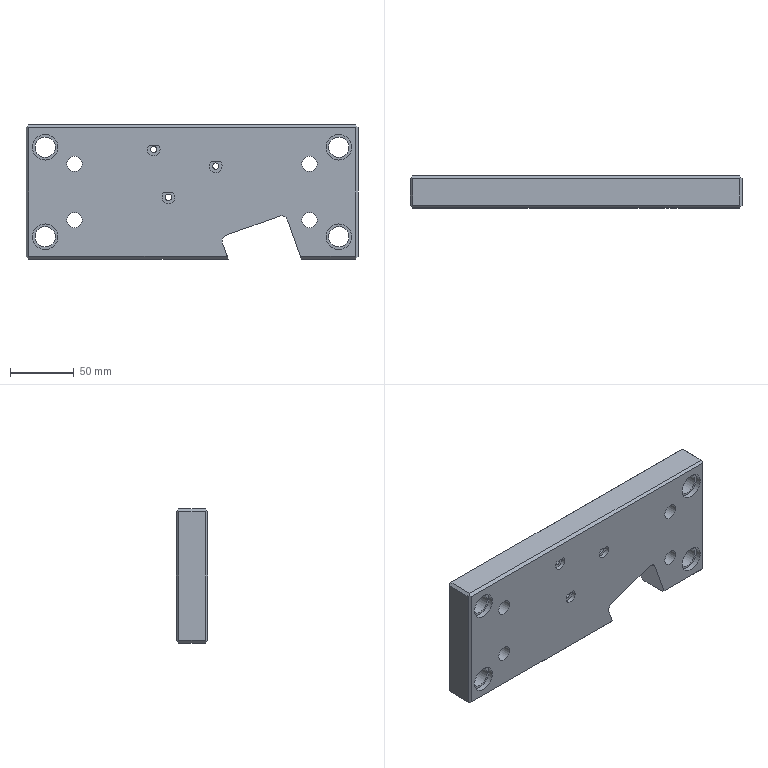Part | STEP file | EJECTION-REMAINER-PLATE_id486_x_t | 1 solid | 54 faces | box 260 x 25 x 105 mm | volume 607320 mm3 | plane 34 | cylinder 20 | commonest cylinder face diameters 10 x5 12 x4 16 x4 20 x4 5 x3
STEP:
#1=CARTESIAN_POINT('',(-129.,-196.5,-51.5));
#2=VERTEX_POINT('',#1);
#3=CARTESIAN_POINT('',(-128.,-197.5,-52.5));
#4=VERTEX_POINT('',#3);
#5=CARTESIAN_POINT('',(-129.,-196.5,-51.5));
#6=DIRECTION('',(0.5774,-0.5774,-0.5774));
#7=VECTOR('',#6,1.);
#8=LINE('',#5,#7);
#9=EDGE_CURVE('',#2,#4,#8,.T.);
#10=ORIENTED_EDGE('',*,*,#9,.T.);
#11=CARTESIAN_POINT('',(-128.,-218.5,-52.5));
#12=VERTEX_POINT('',#11);
#13=CARTESIAN_POINT('',(-128.,175.5,-52.5));
#14=DIRECTION('',(0.,-1.,0.));
#15=VECTOR('',#14,1.);
#16=LINE('',#13,#15);
#17=EDGE_CURVE('',#4,#12,#16,.T.);
#18=ORIENTED_EDGE('',*,*,#17,.T.);
#19=CARTESIAN_POINT('',(-129.,-219.5,-51.5));
#20=VERTEX_POINT('',#19);
#21=CARTESIAN_POINT('',(-129.,-219.5,-51.5));
#22=DIRECTION('',(0.5774,0.5774,-0.5774));
#23=VECTOR('',#22,1.);
#24=LINE('',#21,#23);
#25=EDGE_CURVE('',#20,#12,#24,.T.);
#26=ORIENTED_EDGE('',*,*,#25,.F.);
#27=CARTESIAN_POINT('',(-130.,-218.5,-50.5));
#28=VERTEX_POINT('',#27);
#29=CARTESIAN_POINT('',(-130.,-218.5,-50.5));
#30=DIRECTION('',(0.5774,-0.5774,-0.5774));
#31=VECTOR('',#30,1.);
#32=LINE('',#29,#31);
#33=EDGE_CURVE('',#28,#20,#32,.T.);
#34=ORIENTED_EDGE('',*,*,#33,.F.);
#35=CARTESIAN_POINT('',(-130.,-197.5,-50.5));
#36=VERTEX_POINT('',#35);
#37=CARTESIAN_POINT('',(-130.,-195.5,-50.5));
#38=DIRECTION('',(0.,-1.,0.));
#39=VECTOR('',#38,1.);
#40=LINE('',#37,#39);
#41=EDGE_CURVE('',#36,#28,#40,.T.);
#42=ORIENTED_EDGE('',*,*,#41,.F.);
#43=CARTESIAN_POINT('',(-130.,-197.5,-50.5));
#44=DIRECTION('',(0.5774,0.5774,-0.5774));
#45=VECTOR('',#44,1.);
#46=LINE('',#43,#45);
#47=EDGE_CURVE('',#36,#2,#46,.T.);
#48=ORIENTED_EDGE('',*,*,#47,.T.);
#49=EDGE_LOOP('',(#10,#18,#26,#34,#42,#48));
#50=FACE_OUTER_BOUND('',#49,.T.);
#51=CARTESIAN_POINT('',(-128.,-197.5,-52.5));
#52=DIRECTION('',(-0.7071,0.,-0.7071));
#53=DIRECTION('',(-0.7071,0.,0.7071));
#54=AXIS2_PLACEMENT_3D('',#51,#52,#53);
#55=PLANE('',#54);
#56=ADVANCED_FACE('',(#50),#55,.T.);
#57=CARTESIAN_POINT('',(-130.,-197.5,50.5));
#58=VERTEX_POINT('',#57);
#59=CARTESIAN_POINT('',(-129.,-196.5,51.5));
#60=VERTEX_POINT('',#59);
#61=CARTESIAN_POINT('',(-130.,-197.5,50.5));
#62=DIRECTION('',(0.5774,0.5774,0.5774));
#63=VECTOR('',#62,1.);
#64=LINE('',#61,#63);
#65=EDGE_CURVE('',#58,#60,#64,.T.);
#66=ORIENTED_EDGE('',*,*,#65,.F.);
#67=CARTESIAN_POINT('',(-130.,-218.5,50.5));
#68=VERTEX_POINT('',#67);
#69=CARTESIAN_POINT('',(-130.,-195.5,50.5));
#70=DIRECTION('',(0.,1.,0.));
#71=VECTOR('',#70,1.);
#72=LINE('',#69,#71);
#73=EDGE_CURVE('',#68,#58,#72,.T.);
#74=ORIENTED_EDGE('',*,*,#73,.F.);
#75=CARTESIAN_POINT('',(-129.,-219.5,51.5));
#76=VERTEX_POINT('',#75);
#77=CARTESIAN_POINT('',(-129.,-219.5,51.5));
#78=DIRECTION('',(-0.5774,0.5774,-0.5774));
#79=VECTOR('',#78,1.);
#80=LINE('',#77,#79);
#81=EDGE_CURVE('',#76,#68,#80,.T.);
#82=ORIENTED_EDGE('',*,*,#81,.F.);
#83=CARTESIAN_POINT('',(-128.,-218.5,52.5));
#84=VERTEX_POINT('',#83);
#85=CARTESIAN_POINT('',(-129.,-219.5,51.5));
#86=DIRECTION('',(0.5774,0.5774,0.5774));
#87=VECTOR('',#86,1.);
#88=LINE('',#85,#87);
#89=EDGE_CURVE('',#76,#84,#88,.T.);
#90=ORIENTED_EDGE('',*,*,#89,.T.);
#91=CARTESIAN_POINT('',(-128.,-197.5,52.5));
#92=VERTEX_POINT('',#91);
#93=CARTESIAN_POINT('',(-128.,175.5,52.5));
#94=DIRECTION('',(0.,-1.,0.));
#95=VECTOR('',#94,1.);
#96=LINE('',#93,#95);
#97=EDGE_CURVE('',#92,#84,#96,.T.);
#98=ORIENTED_EDGE('',*,*,#97,.F.);
#99=CARTESIAN_POINT('',(-129.,-196.5,51.5));
#100=DIRECTION('',(0.5774,-0.5774,0.5774));
#101=VECTOR('',#100,1.);
#102=LINE('',#99,#101);
#103=EDGE_CURVE('',#60,#92,#102,.T.);
#104=ORIENTED_EDGE('',*,*,#103,.F.);
#105=EDGE_LOOP('',(#66,#74,#82,#90,#98,#104));
#106=FACE_OUTER_BOUND('',#105,.T.);
#107=CARTESIAN_POINT('',(-128.,-197.5,52.5));
#108=DIRECTION('',(0.7071,0.,-0.7071));
#109=DIRECTION('',(-0.7071,0.,-0.7071));
#110=AXIS2_PLACEMENT_3D('',#107,#108,#109);
#111=PLANE('',#110);
#112=ADVANCED_FACE('',(#106),#111,.F.);
#113=CARTESIAN_POINT('',(130.,-218.5,50.5));
#114=VERTEX_POINT('',#113);
#115=CARTESIAN_POINT('',(129.,-219.5,51.5));
#116=VERTEX_POINT('',#115);
#117=CARTESIAN_POINT('',(130.,-218.5,50.5));
#118=DIRECTION('',(-0.5774,-0.5774,0.5774));
#119=VECTOR('',#118,1.);
#120=LINE('',#117,#119);
#121=EDGE_CURVE('',#114,#116,#120,.T.);
#122=ORIENTED_EDGE('',*,*,#121,.F.);
#123=CARTESIAN_POINT('',(130.,-197.5,50.5));
#124=VERTEX_POINT('',#123);
#125=CARTESIAN_POINT('',(130.,-220.5,50.5));
#126=DIRECTION('',(0.,-1.,0.));
#127=VECTOR('',#126,1.);
#128=LINE('',#125,#127);
#129=EDGE_CURVE('',#124,#114,#128,.T.);
#130=ORIENTED_EDGE('',*,*,#129,.F.);
#131=CARTESIAN_POINT('',(129.,-196.5,51.5));
#132=VERTEX_POINT('',#131);
#133=CARTESIAN_POINT('',(129.,-196.5,51.5));
#134=DIRECTION('',(0.5774,-0.5774,-0.5774));
#135=VECTOR('',#134,1.);
#136=LINE('',#133,#135);
#137=EDGE_CURVE('',#132,#124,#136,.T.);
#138=ORIENTED_EDGE('',*,*,#137,.F.);
#139=CARTESIAN_POINT('',(128.,-197.5,52.5));
#140=VERTEX_POINT('',#139);
#141=CARTESIAN_POINT('',(128.,-197.5,52.5));
#142=DIRECTION('',(0.5774,0.5774,-0.5774));
#143=VECTOR('',#142,1.);
#144=LINE('',#141,#143);
#145=EDGE_CURVE('',#140,#132,#144,.T.);
#146=ORIENTED_EDGE('',*,*,#145,.F.);
#147=CARTESIAN_POINT('',(128.,-218.5,52.5));
#148=VERTEX_POINT('',#147);
#149=CARTESIAN_POINT('',(128.,175.5,52.5));
#150=DIRECTION('',(0.,1.,0.));
#151=VECTOR('',#150,1.);
#152=LINE('',#149,#151);
#153=EDGE_CURVE('',#148,#140,#152,.T.);
#154=ORIENTED_EDGE('',*,*,#153,.F.);
#155=CARTESIAN_POINT('',(128.,-218.5,52.5));
#156=DIRECTION('',(0.5774,-0.5774,-0.5774));
#157=VECTOR('',#156,1.);
#158=LINE('',#155,#157);
#159=EDGE_CURVE('',#148,#116,#158,.T.);
#160=ORIENTED_EDGE('',*,*,#159,.T.);
#161=EDGE_LOOP('',(#122,#130,#138,#146,#154,#160));
#162=FACE_OUTER_BOUND('',#161,.T.);
#163=CARTESIAN_POINT('',(128.,-220.5,52.5));
#164=DIRECTION('',(-0.7071,0.,-0.7071));
#165=DIRECTION('',(-0.7071,0.,0.7071));
#166=AXIS2_PLACEMENT_3D('',#163,#164,#165);
#167=PLANE('',#166);
#168=ADVANCED_FACE('',(#162),#167,.F.);
#169=CARTESIAN_POINT('',(128.,-218.5,-52.5));
#170=VERTEX_POINT('',#169);
#171=CARTESIAN_POINT('',(129.,-219.5,-51.5));
#172=VERTEX_POINT('',#171);
#173=CARTESIAN_POINT('',(128.,-218.5,-52.5));
#174=DIRECTION('',(0.5774,-0.5774,0.5774));
#175=VECTOR('',#174,1.);
#176=LINE('',#173,#175);
#177=EDGE_CURVE('',#170,#172,#176,.T.);
#178=ORIENTED_EDGE('',*,*,#177,.F.);
#179=CARTESIAN_POINT('',(128.,-197.5,-52.5));
#180=VERTEX_POINT('',#179);
#181=CARTESIAN_POINT('',(128.,175.5,-52.5));
#182=DIRECTION('',(0.,1.,0.));
#183=VECTOR('',#182,1.);
#184=LINE('',#181,#183);
#185=EDGE_CURVE('',#170,#180,#184,.T.);
#186=ORIENTED_EDGE('',*,*,#185,.T.);
#187=CARTESIAN_POINT('',(129.,-196.5,-51.5));
#188=VERTEX_POINT('',#187);
#189=CARTESIAN_POINT('',(128.,-197.5,-52.5));
#190=DIRECTION('',(0.5774,0.5774,0.5774));
#191=VECTOR('',#190,1.);
#192=LINE('',#189,#191);
#193=EDGE_CURVE('',#180,#188,#192,.T.);
#194=ORIENTED_EDGE('',*,*,#193,.T.);
#195=CARTESIAN_POINT('',(130.,-197.5,-50.5));
#196=VERTEX_POINT('',#195);
#197=CARTESIAN_POINT('',(129.,-196.5,-51.5));
#198=DIRECTION('',(0.5774,-0.5774,0.5774));
#199=VECTOR('',#198,1.);
#200=LINE('',#197,#199);
#201=EDGE_CURVE('',#188,#196,#200,.T.);
#202=ORIENTED_EDGE('',*,*,#201,.T.);
#203=CARTESIAN_POINT('',(130.,-218.5,-50.5));
#204=VERTEX_POINT('',#203);
#205=CARTESIAN_POINT('',(130.,-220.5,-50.5));
#206=DIRECTION('',(0.,1.,0.));
#207=VECTOR('',#206,1.);
#208=LINE('',#205,#207);
#209=EDGE_CURVE('',#204,#196,#208,.T.);
#210=ORIENTED_EDGE('',*,*,#209,.F.);
#211=CARTESIAN_POINT('',(129.,-219.5,-51.5));
#212=DIRECTION('',(0.5774,0.5774,0.5774));
#213=VECTOR('',#212,1.);
#214=LINE('',#211,#213);
#215=EDGE_CURVE('',#172,#204,#214,.T.);
#216=ORIENTED_EDGE('',*,*,#215,.F.);
#217=EDGE_LOOP('',(#178,#186,#194,#202,#210,#216));
#218=FACE_OUTER_BOUND('',#217,.T.);
#219=CARTESIAN_POINT('',(128.,-220.5,-52.5));
#220=DIRECTION('',(0.7071,0.,-0.7071));
#221=DIRECTION('',(-0.7071,0.,-0.7071));
#222=AXIS2_PLACEMENT_3D('',#219,#220,#221);
#223=PLANE('',#222);
#224=ADVANCED_FACE('',(#218),#223,.T.);
#225=ORIENTED_EDGE('',*,*,#215,.T.);
#226=CARTESIAN_POINT('',(130.,-218.5,-52.5));
#227=DIRECTION('',(0.,0.,-1.));
#228=VECTOR('',#227,1.);
#229=LINE('',#226,#228);
#230=EDGE_CURVE('',#114,#204,#229,.T.);
#231=ORIENTED_EDGE('',*,*,#230,.F.);
#232=ORIENTED_EDGE('',*,*,#121,.T.);
#233=CARTESIAN_POINT('',(128.,-220.5,50.5));
#234=VERTEX_POINT('',#233);
#235=CARTESIAN_POINT('',(129.,-219.5,51.5));
#236=DIRECTION('',(-0.5774,-0.5774,-0.5774));
#237=VECTOR('',#236,1.);
#238=LINE('',#235,#237);
#239=EDGE_CURVE('',#116,#234,#238,.T.);
#240=ORIENTED_EDGE('',*,*,#239,.T.);
#241=CARTESIAN_POINT('',(128.,-220.5,-50.5));
#242=VERTEX_POINT('',#241);
#243=CARTESIAN_POINT('',(128.,-220.5,-52.5));
#244=DIRECTION('',(0.,0.,1.));
#245=VECTOR('',#244,1.);
#246=LINE('',#243,#245);
#247=EDGE_CURVE('',#242,#234,#246,.T.);
#248=ORIENTED_EDGE('',*,*,#247,.F.);
#249=CARTESIAN_POINT('',(129.,-219.5,-51.5));
#250=DIRECTION('',(-0.5774,-0.5774,0.5774));
#251=VECTOR('',#250,1.);
#252=LINE('',#249,#251);
#253=EDGE_CURVE('',#172,#242,#252,.T.);
#254=ORIENTED_EDGE('',*,*,#253,.F.);
#255=EDGE_LOOP('',(#225,#231,#232,#240,#248,#254));
#256=FACE_OUTER_BOUND('',#255,.T.);
#257=CARTESIAN_POINT('',(130.,-218.5,-50.5));
#258=DIRECTION('',(0.7071,-0.7071,0.));
#259=DIRECTION('',(0.7071,0.7071,0.));
#260=AXIS2_PLACEMENT_3D('',#257,#258,#259);
#261=PLANE('',#260);
#262=ADVANCED_FACE('',(#256),#261,.T.);
#263=CARTESIAN_POINT('',(-128.,-220.5,50.5));
#264=VERTEX_POINT('',#263);
#265=CARTESIAN_POINT('',(-128.,-220.5,50.5));
#266=DIRECTION('',(-0.5774,0.5774,0.5774));
#267=VECTOR('',#266,1.);
#268=LINE('',#265,#267);
#269=EDGE_CURVE('',#264,#76,#268,.T.);
#270=ORIENTED_EDGE('',*,*,#269,.F.);
#271=CARTESIAN_POINT('',(-130.,-220.5,50.5));
#272=DIRECTION('',(-1.,0.,0.));
#273=VECTOR('',#272,1.);
#274=LINE('',#271,#273);
#275=EDGE_CURVE('',#234,#264,#274,.T.);
#276=ORIENTED_EDGE('',*,*,#275,.F.);
#277=ORIENTED_EDGE('',*,*,#239,.F.);
#278=ORIENTED_EDGE('',*,*,#159,.F.);
#279=CARTESIAN_POINT('',(-225.,-218.5,52.5));
#280=DIRECTION('',(1.,0.,0.));
#281=VECTOR('',#280,1.);
#282=LINE('',#279,#281);
#283=EDGE_CURVE('',#84,#148,#282,.T.);
#284=ORIENTED_EDGE('',*,*,#283,.F.);
#285=ORIENTED_EDGE('',*,*,#89,.F.);
#286=EDGE_LOOP('',(#270,#276,#277,#278,#284,#285));
#287=FACE_OUTER_BOUND('',#286,.T.);
#288=CARTESIAN_POINT('',(-130.,-218.5,52.5));
#289=DIRECTION('',(0.,0.7071,-0.7071));
#290=DIRECTION('',(0.,0.7071,0.7071));
#291=AXIS2_PLACEMENT_3D('',#288,#289,#290);
#292=PLANE('',#291);
#293=ADVANCED_FACE('',(#287),#292,.F.);
#294=CARTESIAN_POINT('',(-128.,-220.5,-50.5));
#295=VERTEX_POINT('',#294);
#296=CARTESIAN_POINT('',(-128.,-220.5,-50.5));
#297=DIRECTION('',(-0.5774,0.5774,-0.5774));
#298=VECTOR('',#297,1.);
#299=LINE('',#296,#298);
#300=EDGE_CURVE('',#295,#20,#299,.T.);
#301=ORIENTED_EDGE('',*,*,#300,.F.);
#302=CARTESIAN_POINT('',(-128.,-220.5,-52.5));
#303=DIRECTION('',(0.,0.,-1.));
#304=VECTOR('',#303,1.);
#305=LINE('',#302,#304);
#306=EDGE_CURVE('',#264,#295,#305,.T.);
#307=ORIENTED_EDGE('',*,*,#306,.F.);
#308=ORIENTED_EDGE('',*,*,#269,.T.);
#309=ORIENTED_EDGE('',*,*,#81,.T.);
#310=CARTESIAN_POINT('',(-130.,-218.5,-52.5));
#311=DIRECTION('',(0.,0.,1.));
#312=VECTOR('',#311,1.);
#313=LINE('',#310,#312);
#314=EDGE_CURVE('',#28,#68,#313,.T.);
#315=ORIENTED_EDGE('',*,*,#314,.F.);
#316=ORIENTED_EDGE('',*,*,#33,.T.);
#317=EDGE_LOOP('',(#301,#307,#308,#309,#315,#316));
#318=FACE_OUTER_BOUND('',#317,.T.);
#319=CARTESIAN_POINT('',(-128.,-220.5,-50.5));
#320=DIRECTION('',(-0.7071,-0.7071,0.));
#321=DIRECTION('',(0.7071,-0.7071,0.));
#322=AXIS2_PLACEMENT_3D('',#319,#320,#321);
#323=PLANE('',#322);
#324=ADVANCED_FACE('',(#318),#323,.T.);
#325=CARTESIAN_POINT('',(22.131,-217.5,23.73));
#326=VERTEX_POINT('',#325);
#327=CARTESIAN_POINT('',(14.989,-217.5,23.73));
#328=VERTEX_POINT('',#327);
#329=CARTESIAN_POINT('',(18.56,-217.5,20.23));
#330=DIRECTION('',(0.,1.,0.));
#331=DIRECTION('',(0.,0.,1.));
#332=AXIS2_PLACEMENT_3D('',#329,#330,#331);
#333=CIRCLE('',#332,5.);
#334=EDGE_CURVE('',#326,#328,#333,.T.);
#335=ORIENTED_EDGE('',*,*,#334,.T.);
#336=CARTESIAN_POINT('',(14.989,-220.5,23.73));
#337=VERTEX_POINT('',#336);
#338=CARTESIAN_POINT('',(14.989,-220.5,23.73));
#339=DIRECTION('',(0.,-1.,0.));
#340=VECTOR('',#339,1.);
#341=LINE('',#338,#340);
#342=EDGE_CURVE('',#328,#337,#341,.T.);
#343=ORIENTED_EDGE('',*,*,#342,.T.);
#344=CARTESIAN_POINT('',(22.131,-220.5,23.73));
#345=VERTEX_POINT('',#344);
#346=CARTESIAN_POINT('',(18.56,-220.5,20.23));
#347=DIRECTION('',(0.,1.,0.));
#348=DIRECTION('',(0.,0.,1.));
#349=AXIS2_PLACEMENT_3D('',#346,#347,#348);
#350=CIRCLE('',#349,5.);
#351=EDGE_CURVE('',#345,#337,#350,.T.);
#352=ORIENTED_EDGE('',*,*,#351,.F.);
#353=CARTESIAN_POINT('',(22.131,-220.5,23.73));
#354=DIRECTION('',(0.,1.,0.));
#355=VECTOR('',#354,1.);
#356=LINE('',#353,#355);
#357=EDGE_CURVE('',#345,#326,#356,.T.);
#358=ORIENTED_EDGE('',*,*,#357,.T.);
#359=EDGE_LOOP('',(#335,#343,#352,#358));
#360=FACE_OUTER_BOUND('',#359,.T.);
#361=CARTESIAN_POINT('',(18.56,-220.5,20.23));
#362=DIRECTION('',(0.,1.,0.));
#363=DIRECTION('',(0.,0.,1.));
#364=AXIS2_PLACEMENT_3D('',#361,#362,#363);
#365=CYLINDRICAL_SURFACE('',#364,5.);
#366=ADVANCED_FACE('',(#360),#365,.F.);
#367=CARTESIAN_POINT('',(130.,-217.5,23.73));
#368=DIRECTION('',(1.,0.,0.));
#369=VECTOR('',#368,1.);
#370=LINE('',#367,#369);
#371=EDGE_CURVE('',#328,#326,#370,.T.);
#372=ORIENTED_EDGE('',*,*,#371,.T.);
#373=ORIENTED_EDGE('',*,*,#357,.F.);
#374=CARTESIAN_POINT('',(-130.,-220.5,23.73));
#375=DIRECTION('',(1.,0.,0.));
#376=VECTOR('',#375,1.);
#377=LINE('',#374,#376);
#378=EDGE_CURVE('',#337,#345,#377,.T.);
#379=ORIENTED_EDGE('',*,*,#378,.F.);
#380=ORIENTED_EDGE('',*,*,#342,.F.);
#381=EDGE_LOOP('',(#372,#373,#379,#380));
#382=FACE_OUTER_BOUND('',#381,.T.);
#383=CARTESIAN_POINT('',(14.989,-220.5,23.73));
#384=DIRECTION('',(0.,0.,1.));
#385=DIRECTION('',(1.,0.,0.));
#386=AXIS2_PLACEMENT_3D('',#383,#384,#385);
#387=PLANE('',#386);
#388=ADVANCED_FACE('',(#382),#387,.F.);
#389=CARTESIAN_POINT('',(-26.429,-217.5,36.73));
#390=VERTEX_POINT('',#389);
#391=CARTESIAN_POINT('',(-33.571,-217.5,36.73));
#392=VERTEX_POINT('',#391);
#393=CARTESIAN_POINT('',(-30.,-217.5,33.23));
#394=DIRECTION('',(0.,1.,0.));
#395=DIRECTION('',(0.,0.,1.));
#396=AXIS2_PLACEMENT_3D('',#393,#394,#395);
#397=CIRCLE('',#396,5.);
#398=EDGE_CURVE('',#390,#392,#397,.T.);
#399=ORIENTED_EDGE('',*,*,#398,.T.);
#400=CARTESIAN_POINT('',(-33.571,-220.5,36.73));
#401=VERTEX_POINT('',#400);
#402=CARTESIAN_POINT('',(-33.571,-220.5,36.73));
#403=DIRECTION('',(0.,-1.,0.));
#404=VECTOR('',#403,1.);
#405=LINE('',#402,#404);
#406=EDGE_CURVE('',#392,#401,#405,.T.);
#407=ORIENTED_EDGE('',*,*,#406,.T.);
#408=CARTESIAN_POINT('',(-26.429,-220.5,36.73));
#409=VERTEX_POINT('',#408);
#410=CARTESIAN_POINT('',(-30.,-220.5,33.23));
#411=DIRECTION('',(0.,1.,0.));
#412=DIRECTION('',(0.,0.,1.));
#413=AXIS2_PLACEMENT_3D('',#410,#411,#412);
#414=CIRCLE('',#413,5.);
#415=EDGE_CURVE('',#409,#401,#414,.T.);
#416=ORIENTED_EDGE('',*,*,#415,.F.);
#417=CARTESIAN_POINT('',(-26.429,-220.5,36.73));
#418=DIRECTION('',(0.,1.,0.));
#419=VECTOR('',#418,1.);
#420=LINE('',#417,#419);
#421=EDGE_CURVE('',#409,#390,#420,.T.);
#422=ORIENTED_EDGE('',*,*,#421,.T.);
#423=EDGE_LOOP('',(#399,#407,#416,#422));
#424=FACE_OUTER_BOUND('',#423,.T.);
#425=CARTESIAN_POINT('',(-30.,-220.5,33.23));
#426=DIRECTION('',(0.,1.,0.));
#427=DIRECTION('',(0.,0.,1.));
#428=AXIS2_PLACEMENT_3D('',#425,#426,#427);
#429=CYLINDRICAL_SURFACE('',#428,5.);
#430=ADVANCED_FACE('',(#424),#429,.F.);
#431=CARTESIAN_POINT('',(130.,-217.5,36.73));
#432=DIRECTION('',(1.,0.,0.));
#433=VECTOR('',#432,1.);
#434=LINE('',#431,#433);
#435=EDGE_CURVE('',#392,#390,#434,.T.);
#436=ORIENTED_EDGE('',*,*,#435,.T.);
#437=ORIENTED_EDGE('',*,*,#421,.F.);
#438=CARTESIAN_POINT('',(-130.,-220.5,36.73));
#439=DIRECTION('',(1.,0.,0.));
#440=VECTOR('',#439,1.);
#441=LINE('',#438,#440);
#442=EDGE_CURVE('',#401,#409,#441,.T.);
#443=ORIENTED_EDGE('',*,*,#442,.F.);
#444=ORIENTED_EDGE('',*,*,#406,.F.);
#445=EDGE_LOOP('',(#436,#437,#443,#444));
#446=FACE_OUTER_BOUND('',#445,.T.);
#447=CARTESIAN_POINT('',(-33.571,-220.5,36.73));
#448=DIRECTION('',(0.,0.,1.));
#449=DIRECTION('',(1.,0.,0.));
#450=AXIS2_PLACEMENT_3D('',#447,#448,#449);
#451=PLANE('',#450);
#452=ADVANCED_FACE('',(#446),#451,.F.);
#453=CARTESIAN_POINT('',(-14.919,-217.5,-0.58));
#454=VERTEX_POINT('',#453);
#455=CARTESIAN_POINT('',(-22.061,-217.5,-0.58));
#456=VERTEX_POINT('',#455);
#457=CARTESIAN_POINT('',(-18.49,-217.5,-4.08));
#458=DIRECTION('',(0.,1.,0.));
#459=DIRECTION('',(0.,0.,1.));
#460=AXIS2_PLACEMENT_3D('',#457,#458,#459);
#461=CIRCLE('',#460,5.);
#462=EDGE_CURVE('',#454,#456,#461,.T.);
#463=ORIENTED_EDGE('',*,*,#462,.T.);
#464=CARTESIAN_POINT('',(-22.061,-220.5,-0.58));
#465=VERTEX_POINT('',#464);
#466=CARTESIAN_POINT('',(-22.061,-220.5,-0.58));
#467=DIRECTION('',(0.,-1.,0.));
#468=VECTOR('',#467,1.);
#469=LINE('',#466,#468);
#470=EDGE_CURVE('',#456,#465,#469,.T.);
#471=ORIENTED_EDGE('',*,*,#470,.T.);
#472=CARTESIAN_POINT('',(-14.919,-220.5,-0.58));
#473=VERTEX_POINT('',#472);
#474=CARTESIAN_POINT('',(-18.49,-220.5,-4.08));
#475=DIRECTION('',(0.,1.,0.));
#476=DIRECTION('',(0.,0.,1.));
#477=AXIS2_PLACEMENT_3D('',#474,#475,#476);
#478=CIRCLE('',#477,5.);
#479=EDGE_CURVE('',#473,#465,#478,.T.);
#480=ORIENTED_EDGE('',*,*,#479,.F.);
#481=CARTESIAN_POINT('',(-14.919,-220.5,-0.58));
#482=DIRECTION('',(0.,1.,0.));
#483=VECTOR('',#482,1.);
#484=LINE('',#481,#483);
#485=EDGE_CURVE('',#473,#454,#484,.T.);
#486=ORIENTED_EDGE('',*,*,#485,.T.);
#487=EDGE_LOOP('',(#463,#471,#480,#486));
#488=FACE_OUTER_BOUND('',#487,.T.);
#489=CARTESIAN_POINT('',(-18.49,-220.5,-4.08));
#490=DIRECTION('',(0.,1.,0.));
#491=DIRECTION('',(0.,0.,1.));
#492=AXIS2_PLACEMENT_3D('',#489,#490,#491);
#493=CYLINDRICAL_SURFACE('',#492,5.);
#494=ADVANCED_FACE('',(#488),#493,.F.);
#495=CARTESIAN_POINT('',(130.,-217.5,-0.58));
#496=DIRECTION('',(1.,0.,0.));
#497=VECTOR('',#496,1.);
#498=LINE('',#495,#497);
#499=EDGE_CURVE('',#456,#454,#498,.T.);
#500=ORIENTED_EDGE('',*,*,#499,.T.);
#501=ORIENTED_EDGE('',*,*,#485,.F.);
#502=CARTESIAN_POINT('',(-130.,-220.5,-0.58));
#503=DIRECTION('',(1.,0.,0.));
#504=VECTOR('',#503,1.);
#505=LINE('',#502,#504);
#506=EDGE_CURVE('',#465,#473,#505,.T.);
#507=ORIENTED_EDGE('',*,*,#506,.F.);
#508=ORIENTED_EDGE('',*,*,#470,.F.);
#509=EDGE_LOOP('',(#500,#501,#507,#508));
#510=FACE_OUTER_BOUND('',#509,.T.);
#511=CARTESIAN_POINT('',(-22.061,-220.5,-0.58));
#512=DIRECTION('',(0.,0.,1.));
#513=DIRECTION('',(1.,0.,0.));
#514=AXIS2_PLACEMENT_3D('',#511,#512,#513);
#515=PLANE('',#514);
#516=ADVANCED_FACE('',(#510),#515,.F.);
#517=CARTESIAN_POINT('',(115.,-216.5,-45.));
#518=VERTEX_POINT('',#517);
#519=CARTESIAN_POINT('',(115.,-216.5,-35.));
#520=DIRECTION('',(0.,-1.,0.));
#521=DIRECTION('',(0.,0.,-1.));
#522=AXIS2_PLACEMENT_3D('',#519,#520,#521);
#523=CIRCLE('',#522,10.);
#524=EDGE_CURVE('',#518,#518,#523,.T.);
#525=ORIENTED_EDGE('',*,*,#524,.F.);
#526=EDGE_LOOP('',(#525));
#527=FACE_BOUND('',#526,.T.);
#528=CARTESIAN_POINT('',(115.,-220.5,-45.));
#529=VERTEX_POINT('',#528);
#530=CARTESIAN_POINT('',(115.,-220.5,-35.));
#531=DIRECTION('',(0.,1.,0.));
#532=DIRECTION('',(0.,0.,-1.));
#533=AXIS2_PLACEMENT_3D('',#530,#531,#532);
#534=CIRCLE('',#533,10.);
#535=EDGE_CURVE('',#529,#529,#534,.T.);
#536=ORIENTED_EDGE('',*,*,#535,.F.);
#537=EDGE_LOOP('',(#536));
#538=FACE_BOUND('',#537,.T.);
#539=CARTESIAN_POINT('',(115.,-220.5,-35.));
#540=DIRECTION('',(0.,-1.,0.));
#541=DIRECTION('',(0.,0.,-1.));
#542=AXIS2_PLACEMENT_3D('',#539,#540,#541);
#543=CYLINDRICAL_SURFACE('',#542,10.);
#544=ADVANCED_FACE('',(#527,#538),#543,.F.);
#545=CARTESIAN_POINT('',(115.,-216.5,25.));
#546=VERTEX_POINT('',#545);
#547=CARTESIAN_POINT('',(115.,-216.5,35.));
#548=DIRECTION('',(0.,-1.,0.));
#549=DIRECTION('',(0.,0.,-1.));
#550=AXIS2_PLACEMENT_3D('',#547,#548,#549);
#551=CIRCLE('',#550,10.);
#552=EDGE_CURVE('',#546,#546,#551,.T.);
#553=ORIENTED_EDGE('',*,*,#552,.F.);
#554=EDGE_LOOP('',(#553));
#555=FACE_BOUND('',#554,.T.);
#556=CARTESIAN_POINT('',(115.,-220.5,25.));
#557=VERTEX_POINT('',#556);
#558=CARTESIAN_POINT('',(115.,-220.5,35.));
#559=DIRECTION('',(0.,1.,0.));
#560=DIRECTION('',(0.,0.,-1.));
#561=AXIS2_PLACEMENT_3D('',#558,#559,#560);
#562=CIRCLE('',#561,10.);
#563=EDGE_CURVE('',#557,#557,#562,.T.);
#564=ORIENTED_EDGE('',*,*,#563,.F.);
#565=EDGE_LOOP('',(#564));
#566=FACE_BOUND('',#565,.T.);
#567=CARTESIAN_POINT('',(115.,-220.5,35.));
#568=DIRECTION('',(0.,-1.,0.));
#569=DIRECTION('',(0.,0.,-1.));
#570=AXIS2_PLACEMENT_3D('',#567,#568,#569);
#571=CYLINDRICAL_SURFACE('',#570,10.);
#572=ADVANCED_FACE('',(#555,#566),#571,.F.);
#573=CARTESIAN_POINT('',(-115.,-216.5,-45.));
#574=VERTEX_POINT('',#573);
#575=CARTESIAN_POINT('',(-115.,-216.5,-35.));
#576=DIRECTION('',(0.,-1.,0.));
#577=DIRECTION('',(0.,0.,-1.));
#578=AXIS2_PLACEMENT_3D('',#575,#576,#577);
#579=CIRCLE('',#578,10.);
#580=EDGE_CURVE('',#574,#574,#579,.T.);
#581=ORIENTED_EDGE('',*,*,#580,.F.);
#582=EDGE_LOOP('',(#581));
#583=FACE_BOUND('',#582,.T.);
#584=CARTESIAN_POINT('',(-115.,-220.5,-45.));
#585=VERTEX_POINT('',#584);
#586=CARTESIAN_POINT('',(-115.,-220.5,-35.));
#587=DIRECTION('',(0.,1.,0.));
#588=DIRECTION('',(0.,0.,-1.));
#589=AXIS2_PLACEMENT_3D('',#586,#587,#588);
#590=CIRCLE('',#589,10.);
#591=EDGE_CURVE('',#585,#585,#590,.T.);
#592=ORIENTED_EDGE('',*,*,#591,.F.);
#593=EDGE_LOOP('',(#592));
#594=FACE_BOUND('',#593,.T.);
#595=CARTESIAN_POINT('',(-115.,-220.5,-35.));
#596=DIRECTION('',(0.,-1.,0.));
#597=DIRECTION('',(0.,0.,-1.));
#598=AXIS2_PLACEMENT_3D('',#595,#596,#597);
#599=CYLINDRICAL_SURFACE('',#598,10.);
#600=ADVANCED_FACE('',(#583,#594),#599,.F.);
#601=CARTESIAN_POINT('',(-115.,-216.5,25.));
#602=VERTEX_POINT('',#601);
#603=CARTESIAN_POINT('',(-115.,-216.5,35.));
#604=DIRECTION('',(0.,-1.,0.));
#605=DIRECTION('',(0.,0.,-1.));
#606=AXIS2_PLACEMENT_3D('',#603,#604,#605);
#607=CIRCLE('',#606,10.);
#608=EDGE_CURVE('',#602,#602,#607,.T.);
#609=ORIENTED_EDGE('',*,*,#608,.F.);
#610=EDGE_LOOP('',(#609));
#611=FACE_BOUND('',#610,.T.);
#612=CARTESIAN_POINT('',(-115.,-220.5,25.));
#613=VERTEX_POINT('',#612);
#614=CARTESIAN_POINT('',(-115.,-220.5,35.));
#615=DIRECTION('',(0.,1.,0.));
#616=DIRECTION('',(0.,0.,-1.));
#617=AXIS2_PLACEMENT_3D('',#614,#615,#616);
#618=CIRCLE('',#617,10.);
#619=EDGE_CURVE('',#613,#613,#618,.T.);
#620=ORIENTED_EDGE('',*,*,#619,.F.);
#621=EDGE_LOOP('',(#620));
#622=FACE_BOUND('',#621,.T.);
#623=CARTESIAN_POINT('',(-115.,-220.5,35.));
#624=DIRECTION('',(0.,-1.,0.));
#625=DIRECTION('',(0.,0.,-1.));
#626=AXIS2_PLACEMENT_3D('',#623,#624,#625);
#627=CYLINDRICAL_SURFACE('',#626,10.);
#628=ADVANCED_FACE('',(#611,#622),#627,.F.);
#629=CARTESIAN_POINT('',(84.943,-220.5,-50.5));
#630=VERTEX_POINT('',#629);
#631=CARTESIAN_POINT('',(85.651,-218.5,-52.5));
#632=VERTEX_POINT('',#631);
#633=CARTESIAN_POINT('',(84.943,-220.5,-50.5));
#634=DIRECTION('',(0.2429,0.6859,-0.6859));
#635=VECTOR('',#634,1.);
#636=LINE('',#633,#635);
#637=EDGE_CURVE('',#630,#632,#636,.T.);
#638=ORIENTED_EDGE('',*,*,#637,.T.);
#639=CARTESIAN_POINT('',(-225.,-218.5,-52.5));
#640=DIRECTION('',(1.,0.,0.));
#641=VECTOR('',#640,1.);
#642=LINE('',#639,#641);
#643=EDGE_CURVE('',#632,#170,#642,.T.);
#644=ORIENTED_EDGE('',*,*,#643,.T.);
#645=ORIENTED_EDGE('',*,*,#177,.T.);
#646=ORIENTED_EDGE('',*,*,#253,.T.);
#647=CARTESIAN_POINT('',(-130.,-220.5,-50.5));
#648=DIRECTION('',(1.,0.,0.));
#649=VECTOR('',#648,1.);
#650=LINE('',#647,#649);
#651=EDGE_CURVE('',#630,#242,#650,.T.);
#652=ORIENTED_EDGE('',*,*,#651,.F.);
#653=EDGE_LOOP('',(#638,#644,#645,#646,#652));
#654=FACE_OUTER_BOUND('',#653,.T.);
#655=CARTESIAN_POINT('',(-128.,-218.5,-52.5));
#656=DIRECTION('',(0.,-0.7071,-0.7071));
#657=DIRECTION('',(0.,0.7071,-0.7071));
#658=AXIS2_PLACEMENT_3D('',#655,#656,#657);
#659=PLANE('',#658);
#660=ADVANCED_FACE('',(#654),#659,.T.);
#661=ORIENTED_EDGE('',*,*,#25,.T.);
#662=CARTESIAN_POINT('',(28.365,-218.5,-52.5));
#663=VERTEX_POINT('',#662);
#664=CARTESIAN_POINT('',(-225.,-218.5,-52.5));
#665=DIRECTION('',(1.,0.,0.));
#666=VECTOR('',#665,1.);
#667=LINE('',#664,#666);
#668=EDGE_CURVE('',#12,#663,#667,.T.);
#669=ORIENTED_EDGE('',*,*,#668,.T.);
#670=CARTESIAN_POINT('',(27.657,-220.5,-50.5));
#671=VERTEX_POINT('',#670);
#672=CARTESIAN_POINT('',(28.365,-218.5,-52.5));
#673=DIRECTION('',(-0.2429,-0.6859,0.6859));
#674=VECTOR('',#673,1.);
#675=LINE('',#672,#674);
#676=EDGE_CURVE('',#663,#671,#675,.T.);
#677=ORIENTED_EDGE('',*,*,#676,.T.);
#678=CARTESIAN_POINT('',(-130.,-220.5,-50.5));
#679=DIRECTION('',(1.,0.,0.));
#680=VECTOR('',#679,1.);
#681=LINE('',#678,#680);
#682=EDGE_CURVE('',#295,#671,#681,.T.);
#683=ORIENTED_EDGE('',*,*,#682,.F.);
#684=ORIENTED_EDGE('',*,*,#300,.T.);
#685=EDGE_LOOP('',(#661,#669,#677,#683,#684));
#686=FACE_OUTER_BOUND('',#685,.T.);
#687=CARTESIAN_POINT('',(-128.,-218.5,-52.5));
#688=DIRECTION('',(0.,-0.7071,-0.7071));
#689=DIRECTION('',(0.,0.7071,-0.7071));
#690=AXIS2_PLACEMENT_3D('',#687,#688,#689);
#691=PLANE('',#690);
#692=ADVANCED_FACE('',(#686),#691,.T.);
#693=ORIENTED_EDGE('',*,*,#668,.F.);
#694=ORIENTED_EDGE('',*,*,#17,.F.);
#695=CARTESIAN_POINT('',(28.365,-197.5,-52.5));
#696=VERTEX_POINT('',#695);
#697=CARTESIAN_POINT('',(128.,-197.5,-52.5));
#698=DIRECTION('',(-1.,0.,0.));
#699=VECTOR('',#698,1.);
#700=LINE('',#697,#699);
#701=EDGE_CURVE('',#696,#4,#700,.T.);
#702=ORIENTED_EDGE('',*,*,#701,.F.);
#703=CARTESIAN_POINT('',(28.365,-195.5,-52.5));
#704=DIRECTION('',(0.,-1.,0.));
#705=VECTOR('',#704,1.);
#706=LINE('',#703,#705);
#707=EDGE_CURVE('',#696,#663,#706,.T.);
#708=ORIENTED_EDGE('',*,*,#707,.T.);
#709=EDGE_LOOP('',(#693,#694,#702,#708));
#710=FACE_OUTER_BOUND('',#709,.T.);
#711=CARTESIAN_POINT('',(-225.,175.5,-52.5));
#712=DIRECTION('',(0.,0.,1.));
#713=DIRECTION('',(1.,0.,0.));
#714=AXIS2_PLACEMENT_3D('',#711,#712,#713);
#715=PLANE('',#714);
#716=ADVANCED_FACE('',(#710),#715,.F.);
#717=CARTESIAN_POINT('',(-130.,-197.5,-52.5));
#718=DIRECTION('',(0.,0.,1.));
#719=VECTOR('',#718,1.);
#720=LINE('',#717,#719);
#721=EDGE_CURVE('',#36,#58,#720,.T.);
#722=ORIENTED_EDGE('',*,*,#721,.F.);
#723=ORIENTED_EDGE('',*,*,#41,.T.);
#724=ORIENTED_EDGE('',*,*,#314,.T.);
#725=ORIENTED_EDGE('',*,*,#73,.T.);
#726=EDGE_LOOP('',(#722,#723,#724,#725));
#727=FACE_OUTER_BOUND('',#726,.T.);
#728=CARTESIAN_POINT('',(-130.,-195.5,-52.5));
#729=DIRECTION('',(-1.,0.,0.));
#730=DIRECTION('',(0.,0.,1.));
#731=AXIS2_PLACEMENT_3D('',#728,#729,#730);
#732=PLANE('',#731);
#733=ADVANCED_FACE('',(#727),#732,.T.);
#734=ORIENTED_EDGE('',*,*,#283,.T.);
#735=ORIENTED_EDGE('',*,*,#153,.T.);
#736=CARTESIAN_POINT('',(128.,-197.5,52.5));
#737=DIRECTION('',(-1.,0.,0.));
#738=VECTOR('',#737,1.);
#739=LINE('',#736,#738);
#740=EDGE_CURVE('',#140,#92,#739,.T.);
#741=ORIENTED_EDGE('',*,*,#740,.T.);
#742=ORIENTED_EDGE('',*,*,#97,.T.);
#743=EDGE_LOOP('',(#734,#735,#741,#742));
#744=FACE_OUTER_BOUND('',#743,.T.);
#745=CARTESIAN_POINT('',(-225.,175.5,52.5));
#746=DIRECTION('',(0.,0.,1.));
#747=DIRECTION('',(1.,0.,0.));
#748=AXIS2_PLACEMENT_3D('',#745,#746,#747);
#749=PLANE('',#748);
#750=ADVANCED_FACE('',(#744),#749,.T.);
#751=ORIENTED_EDGE('',*,*,#230,.T.);
#752=ORIENTED_EDGE('',*,*,#209,.T.);
#753=CARTESIAN_POINT('',(130.,-197.5,-52.5));
#754=DIRECTION('',(0.,0.,-1.));
#755=VECTOR('',#754,1.);
#756=LINE('',#753,#755);
#757=EDGE_CURVE('',#124,#196,#756,.T.);
#758=ORIENTED_EDGE('',*,*,#757,.F.);
#759=ORIENTED_EDGE('',*,*,#129,.T.);
#760=EDGE_LOOP('',(#751,#752,#758,#759));
#761=FACE_OUTER_BOUND('',#760,.T.);
#762=CARTESIAN_POINT('',(130.,-220.5,-52.5));
#763=DIRECTION('',(1.,0.,0.));
#764=DIRECTION('',(0.,0.,-1.));
#765=AXIS2_PLACEMENT_3D('',#762,#763,#764);
#766=PLANE('',#765);
#767=ADVANCED_FACE('',(#761),#766,.T.);
#768=ORIENTED_EDGE('',*,*,#643,.F.);
#769=CARTESIAN_POINT('',(85.651,-197.5,-52.5));
#770=VERTEX_POINT('',#769);
#771=CARTESIAN_POINT('',(85.651,-195.5,-52.5));
#772=DIRECTION('',(0.,1.,0.));
#773=VECTOR('',#772,1.);
#774=LINE('',#771,#773);
#775=EDGE_CURVE('',#632,#770,#774,.T.);
#776=ORIENTED_EDGE('',*,*,#775,.T.);
#777=CARTESIAN_POINT('',(128.,-197.5,-52.5));
#778=DIRECTION('',(-1.,0.,0.));
#779=VECTOR('',#778,1.);
#780=LINE('',#777,#779);
#781=EDGE_CURVE('',#180,#770,#780,.T.);
#782=ORIENTED_EDGE('',*,*,#781,.F.);
#783=ORIENTED_EDGE('',*,*,#185,.F.);
#784=EDGE_LOOP('',(#768,#776,#782,#783));
#785=FACE_OUTER_BOUND('',#784,.T.);
#786=CARTESIAN_POINT('',(-225.,175.5,-52.5));
#787=DIRECTION('',(0.,0.,1.));
#788=DIRECTION('',(1.,0.,0.));
#789=AXIS2_PLACEMENT_3D('',#786,#787,#788);
#790=PLANE('',#789);
#791=ADVANCED_FACE('',(#785),#790,.F.);
#792=ORIENTED_EDGE('',*,*,#591,.T.);
#793=EDGE_LOOP('',(#792));
#794=FACE_BOUND('',#793,.T.);
#795=ORIENTED_EDGE('',*,*,#619,.T.);
#796=EDGE_LOOP('',(#795));
#797=FACE_BOUND('',#796,.T.);
#798=ORIENTED_EDGE('',*,*,#535,.T.);
#799=EDGE_LOOP('',(#798));
#800=FACE_BOUND('',#799,.T.);
#801=ORIENTED_EDGE('',*,*,#563,.T.);
#802=EDGE_LOOP('',(#801));
#803=FACE_BOUND('',#802,.T.);
#804=ORIENTED_EDGE('',*,*,#506,.T.);
#805=ORIENTED_EDGE('',*,*,#479,.T.);
#806=EDGE_LOOP('',(#804,#805));
#807=FACE_BOUND('',#806,.T.);
#808=ORIENTED_EDGE('',*,*,#442,.T.);
#809=ORIENTED_EDGE('',*,*,#415,.T.);
#810=EDGE_LOOP('',(#808,#809));
#811=FACE_BOUND('',#810,.T.);
#812=ORIENTED_EDGE('',*,*,#378,.T.);
#813=ORIENTED_EDGE('',*,*,#351,.T.);
#814=EDGE_LOOP('',(#812,#813));
#815=FACE_BOUND('',#814,.T.);
#816=CARTESIAN_POINT('',(-92.,-220.5,-16.));
#817=VERTEX_POINT('',#816);
#818=CARTESIAN_POINT('',(-92.,-220.5,-22.));
#819=DIRECTION('',(0.,1.,0.));
#820=DIRECTION('',(0.,0.,1.));
#821=AXIS2_PLACEMENT_3D('',#818,#819,#820);
#822=CIRCLE('',#821,6.);
#823=EDGE_CURVE('',#817,#817,#822,.T.);
#824=ORIENTED_EDGE('',*,*,#823,.T.);
#825=EDGE_LOOP('',(#824));
#826=FACE_BOUND('',#825,.T.);
#827=CARTESIAN_POINT('',(-92.,-220.5,28.));
#828=VERTEX_POINT('',#827);
#829=CARTESIAN_POINT('',(-92.,-220.5,22.));
#830=DIRECTION('',(0.,1.,0.));
#831=DIRECTION('',(0.,0.,1.));
#832=AXIS2_PLACEMENT_3D('',#829,#830,#831);
#833=CIRCLE('',#832,6.);
#834=EDGE_CURVE('',#828,#828,#833,.T.);
#835=ORIENTED_EDGE('',*,*,#834,.T.);
#836=EDGE_LOOP('',(#835));
#837=FACE_BOUND('',#836,.T.);
#838=CARTESIAN_POINT('',(92.,-220.5,28.));
#839=VERTEX_POINT('',#838);
#840=CARTESIAN_POINT('',(92.,-220.5,22.));
#841=DIRECTION('',(0.,1.,0.));
#842=DIRECTION('',(0.,0.,1.));
#843=AXIS2_PLACEMENT_3D('',#840,#841,#842);
#844=CIRCLE('',#843,6.);
#845=EDGE_CURVE('',#839,#839,#844,.T.);
#846=ORIENTED_EDGE('',*,*,#845,.T.);
#847=EDGE_LOOP('',(#846));
#848=FACE_BOUND('',#847,.T.);
#849=CARTESIAN_POINT('',(92.,-220.5,-16.));
#850=VERTEX_POINT('',#849);
#851=CARTESIAN_POINT('',(92.,-220.5,-22.));
#852=DIRECTION('',(0.,1.,0.));
#853=DIRECTION('',(0.,0.,1.));
#854=AXIS2_PLACEMENT_3D('',#851,#852,#853);
#855=CIRCLE('',#854,6.);
#856=EDGE_CURVE('',#850,#850,#855,.T.);
#857=ORIENTED_EDGE('',*,*,#856,.T.);
#858=EDGE_LOOP('',(#857));
#859=FACE_BOUND('',#858,.T.);
#860=ORIENTED_EDGE('',*,*,#306,.T.);
#861=ORIENTED_EDGE('',*,*,#682,.T.);
#862=CARTESIAN_POINT('',(23.967,-220.5,-40.081));
#863=VERTEX_POINT('',#862);
#864=CARTESIAN_POINT('',(28.365,-220.5,-52.5));
#865=DIRECTION('',(-0.3338,0.,0.9426));
#866=VECTOR('',#865,1.);
#867=LINE('',#864,#866);
#868=EDGE_CURVE('',#671,#863,#867,.T.);
#869=ORIENTED_EDGE('',*,*,#868,.T.);
#870=CARTESIAN_POINT('',(27.012,-220.5,-33.699));
#871=VERTEX_POINT('',#870);
#872=CARTESIAN_POINT('',(28.681,-220.5,-38.412));
#873=DIRECTION('',(0.,1.,0.));
#874=DIRECTION('',(0.,0.,1.));
#875=AXIS2_PLACEMENT_3D('',#872,#873,#874);
#876=CIRCLE('',#875,5.);
#877=EDGE_CURVE('',#863,#871,#876,.T.);
#878=ORIENTED_EDGE('',*,*,#877,.T.);
#879=CARTESIAN_POINT('',(68.488,-220.5,-19.011));
#880=VERTEX_POINT('',#879);
#881=CARTESIAN_POINT('',(27.012,-220.5,-33.699));
#882=DIRECTION('',(0.9426,0.,0.3338));
#883=VECTOR('',#882,1.);
#884=LINE('',#881,#883);
#885=EDGE_CURVE('',#871,#880,#884,.T.);
#886=ORIENTED_EDGE('',*,*,#885,.T.);
#887=CARTESIAN_POINT('',(74.87,-220.5,-22.055));
#888=VERTEX_POINT('',#887);
#889=CARTESIAN_POINT('',(70.157,-220.5,-23.724));
#890=DIRECTION('',(0.,1.,0.));
#891=DIRECTION('',(0.,0.,1.));
#892=AXIS2_PLACEMENT_3D('',#889,#890,#891);
#893=CIRCLE('',#892,5.);
#894=EDGE_CURVE('',#880,#888,#893,.T.);
#895=ORIENTED_EDGE('',*,*,#894,.T.);
#896=CARTESIAN_POINT('',(74.87,-220.5,-22.055));
#897=DIRECTION('',(0.3338,0.,-0.9426));
#898=VECTOR('',#897,1.);
#899=LINE('',#896,#898);
#900=EDGE_CURVE('',#888,#630,#899,.T.);
#901=ORIENTED_EDGE('',*,*,#900,.T.);
#902=ORIENTED_EDGE('',*,*,#651,.T.);
#903=ORIENTED_EDGE('',*,*,#247,.T.);
#904=ORIENTED_EDGE('',*,*,#275,.T.);
#905=EDGE_LOOP('',(#860,#861,#869,#878,#886,#895,#901,#902,#903,#904));
#906=FACE_BOUND('',#905,.T.);
#907=CARTESIAN_POINT('',(-130.,-220.5,-52.5));
#908=DIRECTION('',(0.,-1.,0.));
#909=DIRECTION('',(0.,0.,-1.));
#910=AXIS2_PLACEMENT_3D('',#907,#908,#909);
#911=PLANE('',#910);
#912=ADVANCED_FACE('',(#794,#797,#800,#803,#807,#811,#815,#826,#837,#848,#859,#906),#911,.T.);
#913=CARTESIAN_POINT('',(18.56,-217.5,22.73));
#914=VERTEX_POINT('',#913);
#915=CARTESIAN_POINT('',(18.56,-217.5,20.23));
#916=DIRECTION('',(0.,1.,0.));
#917=DIRECTION('',(0.,0.,1.));
#918=AXIS2_PLACEMENT_3D('',#915,#916,#917);
#919=CIRCLE('',#918,2.5);
#920=EDGE_CURVE('',#914,#914,#919,.T.);
#921=ORIENTED_EDGE('',*,*,#920,.T.);
#922=EDGE_LOOP('',(#921));
#923=FACE_BOUND('',#922,.T.);
#924=ORIENTED_EDGE('',*,*,#334,.F.);
#925=ORIENTED_EDGE('',*,*,#371,.F.);
#926=EDGE_LOOP('',(#924,#925));
#927=FACE_BOUND('',#926,.T.);
#928=CARTESIAN_POINT('',(130.,-217.5,-52.5));
#929=DIRECTION('',(0.,1.,0.));
#930=DIRECTION('',(0.,0.,1.));
#931=AXIS2_PLACEMENT_3D('',#928,#929,#930);
#932=PLANE('',#931);
#933=ADVANCED_FACE('',(#923,#927),#932,.F.);
#934=CARTESIAN_POINT('',(-30.,-217.5,35.73));
#935=VERTEX_POINT('',#934);
#936=CARTESIAN_POINT('',(-30.,-217.5,33.23));
#937=DIRECTION('',(0.,1.,0.));
#938=DIRECTION('',(0.,0.,1.));
#939=AXIS2_PLACEMENT_3D('',#936,#937,#938);
#940=CIRCLE('',#939,2.5);
#941=EDGE_CURVE('',#935,#935,#940,.T.);
#942=ORIENTED_EDGE('',*,*,#941,.T.);
#943=EDGE_LOOP('',(#942));
#944=FACE_BOUND('',#943,.T.);
#945=ORIENTED_EDGE('',*,*,#398,.F.);
#946=ORIENTED_EDGE('',*,*,#435,.F.);
#947=EDGE_LOOP('',(#945,#946));
#948=FACE_BOUND('',#947,.T.);
#949=CARTESIAN_POINT('',(130.,-217.5,-52.5));
#950=DIRECTION('',(0.,1.,0.));
#951=DIRECTION('',(0.,0.,1.));
#952=AXIS2_PLACEMENT_3D('',#949,#950,#951);
#953=PLANE('',#952);
#954=ADVANCED_FACE('',(#944,#948),#953,.F.);
#955=CARTESIAN_POINT('',(-18.49,-217.5,-1.58));
#956=VERTEX_POINT('',#955);
#957=CARTESIAN_POINT('',(-18.49,-217.5,-4.08));
#958=DIRECTION('',(0.,1.,0.));
#959=DIRECTION('',(0.,0.,1.));
#960=AXIS2_PLACEMENT_3D('',#957,#958,#959);
#961=CIRCLE('',#960,2.5);
#962=EDGE_CURVE('',#956,#956,#961,.T.);
#963=ORIENTED_EDGE('',*,*,#962,.T.);
#964=EDGE_LOOP('',(#963));
#965=FACE_BOUND('',#964,.T.);
#966=ORIENTED_EDGE('',*,*,#462,.F.);
#967=ORIENTED_EDGE('',*,*,#499,.F.);
#968=EDGE_LOOP('',(#966,#967));
#969=FACE_BOUND('',#968,.T.);
#970=CARTESIAN_POINT('',(130.,-217.5,-52.5));
#971=DIRECTION('',(0.,1.,0.));
#972=DIRECTION('',(0.,0.,1.));
#973=AXIS2_PLACEMENT_3D('',#970,#971,#972);
#974=PLANE('',#973);
#975=ADVANCED_FACE('',(#965,#969),#974,.F.);
#976=CARTESIAN_POINT('',(115.,-216.5,-27.));
#977=VERTEX_POINT('',#976);
#978=CARTESIAN_POINT('',(115.,-216.5,-35.));
#979=DIRECTION('',(0.,1.,0.));
#980=DIRECTION('',(0.,0.,1.));
#981=AXIS2_PLACEMENT_3D('',#978,#979,#980);
#982=CIRCLE('',#981,8.);
#983=EDGE_CURVE('',#977,#977,#982,.T.);
#984=ORIENTED_EDGE('',*,*,#983,.T.);
#985=EDGE_LOOP('',(#984));
#986=FACE_BOUND('',#985,.T.);
#987=ORIENTED_EDGE('',*,*,#524,.T.);
#988=EDGE_LOOP('',(#987));
#989=FACE_BOUND('',#988,.T.);
#990=CARTESIAN_POINT('',(-225.,-216.5,-52.5));
#991=DIRECTION('',(0.,-1.,0.));
#992=DIRECTION('',(0.,0.,-1.));
#993=AXIS2_PLACEMENT_3D('',#990,#991,#992);
#994=PLANE('',#993);
#995=ADVANCED_FACE('',(#986,#989),#994,.T.);
#996=CARTESIAN_POINT('',(115.,-216.5,43.));
#997=VERTEX_POINT('',#996);
#998=CARTESIAN_POINT('',(115.,-216.5,35.));
#999=DIRECTION('',(0.,1.,0.));
#1000=DIRECTION('',(0.,0.,1.));
#1001=AXIS2_PLACEMENT_3D('',#998,#999,#1000);
#1002=CIRCLE('',#1001,8.);
#1003=EDGE_CURVE('',#997,#997,#1002,.T.);
#1004=ORIENTED_EDGE('',*,*,#1003,.T.);
#1005=EDGE_LOOP('',(#1004));
#1006=FACE_BOUND('',#1005,.T.);
#1007=ORIENTED_EDGE('',*,*,#552,.T.);
#1008=EDGE_LOOP('',(#1007));
#1009=FACE_BOUND('',#1008,.T.);
#1010=CARTESIAN_POINT('',(-225.,-216.5,-52.5));
#1011=DIRECTION('',(0.,-1.,0.));
#1012=DIRECTION('',(0.,0.,-1.));
#1013=AXIS2_PLACEMENT_3D('',#1010,#1011,#1012);
#1014=PLANE('',#1013);
#1015=ADVANCED_FACE('',(#1006,#1009),#1014,.T.);
#1016=CARTESIAN_POINT('',(-115.,-216.5,-27.));
#1017=VERTEX_POINT('',#1016);
#1018=CARTESIAN_POINT('',(-115.,-216.5,-35.));
#1019=DIRECTION('',(0.,1.,0.));
#1020=DIRECTION('',(0.,0.,1.));
#1021=AXIS2_PLACEMENT_3D('',#1018,#1019,#1020);
#1022=CIRCLE('',#1021,8.);
#1023=EDGE_CURVE('',#1017,#1017,#1022,.T.);
#1024=ORIENTED_EDGE('',*,*,#1023,.T.);
#1025=EDGE_LOOP('',(#1024));
#1026=FACE_BOUND('',#1025,.T.);
#1027=ORIENTED_EDGE('',*,*,#580,.T.);
#1028=EDGE_LOOP('',(#1027));
#1029=FACE_BOUND('',#1028,.T.);
#1030=CARTESIAN_POINT('',(-225.,-216.5,-52.5));
#1031=DIRECTION('',(0.,-1.,0.));
#1032=DIRECTION('',(0.,0.,-1.));
#1033=AXIS2_PLACEMENT_3D('',#1030,#1031,#1032);
#1034=PLANE('',#1033);
#1035=ADVANCED_FACE('',(#1026,#1029),#1034,.T.);
#1036=CARTESIAN_POINT('',(-115.,-216.5,43.));
#1037=VERTEX_POINT('',#1036);
#1038=CARTESIAN_POINT('',(-115.,-216.5,35.));
#1039=DIRECTION('',(0.,1.,0.));
#1040=DIRECTION('',(0.,0.,1.));
#1041=AXIS2_PLACEMENT_3D('',#1038,#1039,#1040);
#1042=CIRCLE('',#1041,8.);
#1043=EDGE_CURVE('',#1037,#1037,#1042,.T.);
#1044=ORIENTED_EDGE('',*,*,#1043,.T.);
#1045=EDGE_LOOP('',(#1044));
#1046=FACE_BOUND('',#1045,.T.);
#1047=ORIENTED_EDGE('',*,*,#608,.T.);
#1048=EDGE_LOOP('',(#1047));
#1049=FACE_BOUND('',#1048,.T.);
#1050=CARTESIAN_POINT('',(-225.,-216.5,-52.5));
#1051=DIRECTION('',(0.,-1.,0.));
#1052=DIRECTION('',(0.,0.,-1.));
#1053=AXIS2_PLACEMENT_3D('',#1050,#1051,#1052);
#1054=PLANE('',#1053);
#1055=ADVANCED_FACE('',(#1046,#1049),#1054,.T.);
#1056=ORIENTED_EDGE('',*,*,#900,.F.);
#1057=CARTESIAN_POINT('',(74.87,-195.5,-22.055));
#1058=VERTEX_POINT('',#1057);
#1059=CARTESIAN_POINT('',(74.87,-195.5,-22.055));
#1060=DIRECTION('',(0.,1.,0.));
#1061=VECTOR('',#1060,1.);
#1062=LINE('',#1059,#1061);
#1063=EDGE_CURVE('',#888,#1058,#1062,.T.);
#1064=ORIENTED_EDGE('',*,*,#1063,.T.);
#1065=CARTESIAN_POINT('',(84.943,-195.5,-50.5));
#1066=VERTEX_POINT('',#1065);
#1067=CARTESIAN_POINT('',(84.943,-195.5,-50.5));
#1068=DIRECTION('',(-0.3338,0.,0.9426));
#1069=VECTOR('',#1068,1.);
#1070=LINE('',#1067,#1069);
#1071=EDGE_CURVE('',#1066,#1058,#1070,.T.);
#1072=ORIENTED_EDGE('',*,*,#1071,.F.);
#1073=CARTESIAN_POINT('',(85.651,-197.5,-52.5));
#1074=DIRECTION('',(-0.2429,0.6859,0.6859));
#1075=VECTOR('',#1074,1.);
#1076=LINE('',#1073,#1075);
#1077=EDGE_CURVE('',#770,#1066,#1076,.T.);
#1078=ORIENTED_EDGE('',*,*,#1077,.F.);
#1079=ORIENTED_EDGE('',*,*,#775,.F.);
#1080=ORIENTED_EDGE('',*,*,#637,.F.);
#1081=EDGE_LOOP('',(#1056,#1064,#1072,#1078,#1079,#1080));
#1082=FACE_OUTER_BOUND('',#1081,.T.);
#1083=CARTESIAN_POINT('',(74.87,-195.5,-22.055));
#1084=DIRECTION('',(0.9426,0.,0.3338));
#1085=DIRECTION('',(0.3338,0.,-0.9426));
#1086=AXIS2_PLACEMENT_3D('',#1083,#1084,#1085);
#1087=PLANE('',#1086);
#1088=ADVANCED_FACE('',(#1082),#1087,.F.);
#1089=ORIENTED_EDGE('',*,*,#894,.F.);
#1090=CARTESIAN_POINT('',(68.488,-195.5,-19.011));
#1091=VERTEX_POINT('',#1090);
#1092=CARTESIAN_POINT('',(68.488,-195.5,-19.011));
#1093=DIRECTION('',(0.,1.,0.));
#1094=VECTOR('',#1093,1.);
#1095=LINE('',#1092,#1094);
#1096=EDGE_CURVE('',#880,#1091,#1095,.T.);
#1097=ORIENTED_EDGE('',*,*,#1096,.T.);
#1098=CARTESIAN_POINT('',(70.157,-195.5,-23.724));
#1099=DIRECTION('',(0.,-1.,0.));
#1100=DIRECTION('',(0.,0.,1.));
#1101=AXIS2_PLACEMENT_3D('',#1098,#1099,#1100);
#1102=CIRCLE('',#1101,5.);
#1103=EDGE_CURVE('',#1058,#1091,#1102,.T.);
#1104=ORIENTED_EDGE('',*,*,#1103,.F.);
#1105=ORIENTED_EDGE('',*,*,#1063,.F.);
#1106=EDGE_LOOP('',(#1089,#1097,#1104,#1105));
#1107=FACE_OUTER_BOUND('',#1106,.T.);
#1108=CARTESIAN_POINT('',(70.157,-195.5,-23.724));
#1109=DIRECTION('',(0.,1.,0.));
#1110=DIRECTION('',(0.,0.,1.));
#1111=AXIS2_PLACEMENT_3D('',#1108,#1109,#1110);
#1112=CYLINDRICAL_SURFACE('',#1111,5.);
#1113=ADVANCED_FACE('',(#1107),#1112,.F.);
#1114=ORIENTED_EDGE('',*,*,#885,.F.);
#1115=CARTESIAN_POINT('',(27.012,-195.5,-33.699));
#1116=VERTEX_POINT('',#1115);
#1117=CARTESIAN_POINT('',(27.012,-195.5,-33.699));
#1118=DIRECTION('',(0.,1.,0.));
#1119=VECTOR('',#1118,1.);
#1120=LINE('',#1117,#1119);
#1121=EDGE_CURVE('',#871,#1116,#1120,.T.);
#1122=ORIENTED_EDGE('',*,*,#1121,.T.);
#1123=CARTESIAN_POINT('',(68.488,-195.5,-19.011));
#1124=DIRECTION('',(-0.9426,0.,-0.3338));
#1125=VECTOR('',#1124,1.);
#1126=LINE('',#1123,#1125);
#1127=EDGE_CURVE('',#1091,#1116,#1126,.T.);
#1128=ORIENTED_EDGE('',*,*,#1127,.F.);
#1129=ORIENTED_EDGE('',*,*,#1096,.F.);
#1130=EDGE_LOOP('',(#1114,#1122,#1128,#1129));
#1131=FACE_OUTER_BOUND('',#1130,.T.);
#1132=CARTESIAN_POINT('',(27.012,-195.5,-33.699));
#1133=DIRECTION('',(-0.3338,0.,0.9426));
#1134=DIRECTION('',(0.9426,0.,0.3338));
#1135=AXIS2_PLACEMENT_3D('',#1132,#1133,#1134);
#1136=PLANE('',#1135);
#1137=ADVANCED_FACE('',(#1131),#1136,.F.);
#1138=ORIENTED_EDGE('',*,*,#877,.F.);
#1139=CARTESIAN_POINT('',(23.967,-195.5,-40.081));
#1140=VERTEX_POINT('',#1139);
#1141=CARTESIAN_POINT('',(23.967,-195.5,-40.081));
#1142=DIRECTION('',(0.,1.,0.));
#1143=VECTOR('',#1142,1.);
#1144=LINE('',#1141,#1143);
#1145=EDGE_CURVE('',#863,#1140,#1144,.T.);
#1146=ORIENTED_EDGE('',*,*,#1145,.T.);
#1147=CARTESIAN_POINT('',(28.681,-195.5,-38.412));
#1148=DIRECTION('',(0.,-1.,0.));
#1149=DIRECTION('',(0.,0.,1.));
#1150=AXIS2_PLACEMENT_3D('',#1147,#1148,#1149);
#1151=CIRCLE('',#1150,5.);
#1152=EDGE_CURVE('',#1116,#1140,#1151,.T.);
#1153=ORIENTED_EDGE('',*,*,#1152,.F.);
#1154=ORIENTED_EDGE('',*,*,#1121,.F.);
#1155=EDGE_LOOP('',(#1138,#1146,#1153,#1154));
#1156=FACE_OUTER_BOUND('',#1155,.T.);
#1157=CARTESIAN_POINT('',(28.681,-195.5,-38.412));
#1158=DIRECTION('',(0.,1.,0.));
#1159=DIRECTION('',(0.,0.,1.));
#1160=AXIS2_PLACEMENT_3D('',#1157,#1158,#1159);
#1161=CYLINDRICAL_SURFACE('',#1160,5.);
#1162=ADVANCED_FACE('',(#1156),#1161,.F.);
#1163=CARTESIAN_POINT('',(27.657,-195.5,-50.5));
#1164=VERTEX_POINT('',#1163);
#1165=CARTESIAN_POINT('',(23.967,-195.5,-40.081));
#1166=DIRECTION('',(0.3338,0.,-0.9426));
#1167=VECTOR('',#1166,1.);
#1168=LINE('',#1165,#1167);
#1169=EDGE_CURVE('',#1140,#1164,#1168,.T.);
#1170=ORIENTED_EDGE('',*,*,#1169,.F.);
#1171=ORIENTED_EDGE('',*,*,#1145,.F.);
#1172=ORIENTED_EDGE('',*,*,#868,.F.);
#1173=ORIENTED_EDGE('',*,*,#676,.F.);
#1174=ORIENTED_EDGE('',*,*,#707,.F.);
#1175=CARTESIAN_POINT('',(27.657,-195.5,-50.5));
#1176=DIRECTION('',(0.2429,-0.6859,-0.6859));
#1177=VECTOR('',#1176,1.);
#1178=LINE('',#1175,#1177);
#1179=EDGE_CURVE('',#1164,#696,#1178,.T.);
#1180=ORIENTED_EDGE('',*,*,#1179,.F.);
#1181=EDGE_LOOP('',(#1170,#1171,#1172,#1173,#1174,#1180));
#1182=FACE_OUTER_BOUND('',#1181,.T.);
#1183=CARTESIAN_POINT('',(28.365,-195.5,-52.5));
#1184=DIRECTION('',(-0.9426,0.,-0.3338));
#1185=DIRECTION('',(-0.3338,0.,0.9426));
#1186=AXIS2_PLACEMENT_3D('',#1183,#1184,#1185);
#1187=PLANE('',#1186);
#1188=ADVANCED_FACE('',(#1182),#1187,.F.);
#1189=ORIENTED_EDGE('',*,*,#1179,.T.);
#1190=ORIENTED_EDGE('',*,*,#701,.T.);
#1191=ORIENTED_EDGE('',*,*,#9,.F.);
#1192=CARTESIAN_POINT('',(-128.,-195.5,-50.5));
#1193=VERTEX_POINT('',#1192);
#1194=CARTESIAN_POINT('',(-128.,-195.5,-50.5));
#1195=DIRECTION('',(-0.5774,-0.5774,-0.5774));
#1196=VECTOR('',#1195,1.);
#1197=LINE('',#1194,#1196);
#1198=EDGE_CURVE('',#1193,#2,#1197,.T.);
#1199=ORIENTED_EDGE('',*,*,#1198,.F.);
#1200=CARTESIAN_POINT('',(130.,-195.5,-50.5));
#1201=DIRECTION('',(-1.,0.,0.));
#1202=VECTOR('',#1201,1.);
#1203=LINE('',#1200,#1202);
#1204=EDGE_CURVE('',#1164,#1193,#1203,.T.);
#1205=ORIENTED_EDGE('',*,*,#1204,.F.);
#1206=EDGE_LOOP('',(#1189,#1190,#1191,#1199,#1205));
#1207=FACE_OUTER_BOUND('',#1206,.T.);
#1208=CARTESIAN_POINT('',(128.,-197.5,-52.5));
#1209=DIRECTION('',(0.,0.7071,-0.7071));
#1210=DIRECTION('',(0.,0.7071,0.7071));
#1211=AXIS2_PLACEMENT_3D('',#1208,#1209,#1210);
#1212=PLANE('',#1211);
#1213=ADVANCED_FACE('',(#1207),#1212,.T.);
#1214=ORIENTED_EDGE('',*,*,#47,.F.);
#1215=ORIENTED_EDGE('',*,*,#721,.T.);
#1216=ORIENTED_EDGE('',*,*,#65,.T.);
#1217=CARTESIAN_POINT('',(-128.,-195.5,50.5));
#1218=VERTEX_POINT('',#1217);
#1219=CARTESIAN_POINT('',(-129.,-196.5,51.5));
#1220=DIRECTION('',(0.5774,0.5774,-0.5774));
#1221=VECTOR('',#1220,1.);
#1222=LINE('',#1219,#1221);
#1223=EDGE_CURVE('',#60,#1218,#1222,.T.);
#1224=ORIENTED_EDGE('',*,*,#1223,.T.);
#1225=CARTESIAN_POINT('',(-128.,-195.5,-52.5));
#1226=DIRECTION('',(0.,0.,1.));
#1227=VECTOR('',#1226,1.);
#1228=LINE('',#1225,#1227);
#1229=EDGE_CURVE('',#1193,#1218,#1228,.T.);
#1230=ORIENTED_EDGE('',*,*,#1229,.F.);
#1231=ORIENTED_EDGE('',*,*,#1198,.T.);
#1232=EDGE_LOOP('',(#1214,#1215,#1216,#1224,#1230,#1231));
#1233=FACE_OUTER_BOUND('',#1232,.T.);
#1234=CARTESIAN_POINT('',(-130.,-197.5,-52.5));
#1235=DIRECTION('',(-0.7071,0.7071,0.));
#1236=DIRECTION('',(-0.7071,-0.7071,0.));
#1237=AXIS2_PLACEMENT_3D('',#1234,#1235,#1236);
#1238=PLANE('',#1237);
#1239=ADVANCED_FACE('',(#1233),#1238,.T.);
#1240=CARTESIAN_POINT('',(128.,-195.5,50.5));
#1241=VERTEX_POINT('',#1240);
#1242=CARTESIAN_POINT('',(128.,-195.5,50.5));
#1243=DIRECTION('',(0.5774,-0.5774,0.5774));
#1244=VECTOR('',#1243,1.);
#1245=LINE('',#1242,#1244);
#1246=EDGE_CURVE('',#1241,#132,#1245,.T.);
#1247=ORIENTED_EDGE('',*,*,#1246,.F.);
#1248=CARTESIAN_POINT('',(130.,-195.5,50.5));
#1249=DIRECTION('',(1.,0.,0.));
#1250=VECTOR('',#1249,1.);
#1251=LINE('',#1248,#1250);
#1252=EDGE_CURVE('',#1218,#1241,#1251,.T.);
#1253=ORIENTED_EDGE('',*,*,#1252,.F.);
#1254=ORIENTED_EDGE('',*,*,#1223,.F.);
#1255=ORIENTED_EDGE('',*,*,#103,.T.);
#1256=ORIENTED_EDGE('',*,*,#740,.F.);
#1257=ORIENTED_EDGE('',*,*,#145,.T.);
#1258=EDGE_LOOP('',(#1247,#1253,#1254,#1255,#1256,#1257));
#1259=FACE_OUTER_BOUND('',#1258,.T.);
#1260=CARTESIAN_POINT('',(128.,-197.5,52.5));
#1261=DIRECTION('',(0.,-0.7071,-0.7071));
#1262=DIRECTION('',(0.,0.7071,-0.7071));
#1263=AXIS2_PLACEMENT_3D('',#1260,#1261,#1262);
#1264=PLANE('',#1263);
#1265=ADVANCED_FACE('',(#1259),#1264,.F.);
#1266=CARTESIAN_POINT('',(128.,-195.5,-50.5));
#1267=VERTEX_POINT('',#1266);
#1268=CARTESIAN_POINT('',(128.,-195.5,-50.5));
#1269=DIRECTION('',(0.5774,-0.5774,-0.5774));
#1270=VECTOR('',#1269,1.);
#1271=LINE('',#1268,#1270);
#1272=EDGE_CURVE('',#1267,#188,#1271,.T.);
#1273=ORIENTED_EDGE('',*,*,#1272,.F.);
#1274=CARTESIAN_POINT('',(128.,-195.5,-52.5));
#1275=DIRECTION('',(0.,0.,-1.));
#1276=VECTOR('',#1275,1.);
#1277=LINE('',#1274,#1276);
#1278=EDGE_CURVE('',#1241,#1267,#1277,.T.);
#1279=ORIENTED_EDGE('',*,*,#1278,.F.);
#1280=ORIENTED_EDGE('',*,*,#1246,.T.);
#1281=ORIENTED_EDGE('',*,*,#137,.T.);
#1282=ORIENTED_EDGE('',*,*,#757,.T.);
#1283=ORIENTED_EDGE('',*,*,#201,.F.);
#1284=EDGE_LOOP('',(#1273,#1279,#1280,#1281,#1282,#1283));
#1285=FACE_OUTER_BOUND('',#1284,.T.);
#1286=CARTESIAN_POINT('',(128.,-195.5,-52.5));
#1287=DIRECTION('',(0.7071,0.7071,0.));
#1288=DIRECTION('',(-0.7071,0.7071,0.));
#1289=AXIS2_PLACEMENT_3D('',#1286,#1287,#1288);
#1290=PLANE('',#1289);
#1291=ADVANCED_FACE('',(#1285),#1290,.T.);
#1292=ORIENTED_EDGE('',*,*,#193,.F.);
#1293=ORIENTED_EDGE('',*,*,#781,.T.);
#1294=ORIENTED_EDGE('',*,*,#1077,.T.);
#1295=CARTESIAN_POINT('',(130.,-195.5,-50.5));
#1296=DIRECTION('',(-1.,0.,0.));
#1297=VECTOR('',#1296,1.);
#1298=LINE('',#1295,#1297);
#1299=EDGE_CURVE('',#1267,#1066,#1298,.T.);
#1300=ORIENTED_EDGE('',*,*,#1299,.F.);
#1301=ORIENTED_EDGE('',*,*,#1272,.T.);
#1302=EDGE_LOOP('',(#1292,#1293,#1294,#1300,#1301));
#1303=FACE_OUTER_BOUND('',#1302,.T.);
#1304=CARTESIAN_POINT('',(128.,-197.5,-52.5));
#1305=DIRECTION('',(0.,0.7071,-0.7071));
#1306=DIRECTION('',(0.,0.7071,0.7071));
#1307=AXIS2_PLACEMENT_3D('',#1304,#1305,#1306);
#1308=PLANE('',#1307);
#1309=ADVANCED_FACE('',(#1303),#1308,.T.);
#1310=ORIENTED_EDGE('',*,*,#856,.F.);
#1311=EDGE_LOOP('',(#1310));
#1312=FACE_BOUND('',#1311,.T.);
#1313=CARTESIAN_POINT('',(92.,-195.5,-16.));
#1314=VERTEX_POINT('',#1313);
#1315=CARTESIAN_POINT('',(92.,-195.5,-22.));
#1316=DIRECTION('',(0.,-1.,0.));
#1317=DIRECTION('',(0.,0.,1.));
#1318=AXIS2_PLACEMENT_3D('',#1315,#1316,#1317);
#1319=CIRCLE('',#1318,6.);
#1320=EDGE_CURVE('',#1314,#1314,#1319,.T.);
#1321=ORIENTED_EDGE('',*,*,#1320,.F.);
#1322=EDGE_LOOP('',(#1321));
#1323=FACE_BOUND('',#1322,.T.);
#1324=CARTESIAN_POINT('',(92.,-195.5,-22.));
#1325=DIRECTION('',(0.,1.,0.));
#1326=DIRECTION('',(0.,0.,1.));
#1327=AXIS2_PLACEMENT_3D('',#1324,#1325,#1326);
#1328=CYLINDRICAL_SURFACE('',#1327,6.);
#1329=ADVANCED_FACE('',(#1312,#1323),#1328,.F.);
#1330=ORIENTED_EDGE('',*,*,#845,.F.);
#1331=EDGE_LOOP('',(#1330));
#1332=FACE_BOUND('',#1331,.T.);
#1333=CARTESIAN_POINT('',(92.,-195.5,28.));
#1334=VERTEX_POINT('',#1333);
#1335=CARTESIAN_POINT('',(92.,-195.5,22.));
#1336=DIRECTION('',(0.,-1.,0.));
#1337=DIRECTION('',(0.,0.,1.));
#1338=AXIS2_PLACEMENT_3D('',#1335,#1336,#1337);
#1339=CIRCLE('',#1338,6.);
#1340=EDGE_CURVE('',#1334,#1334,#1339,.T.);
#1341=ORIENTED_EDGE('',*,*,#1340,.F.);
#1342=EDGE_LOOP('',(#1341));
#1343=FACE_BOUND('',#1342,.T.);
#1344=CARTESIAN_POINT('',(92.,-195.5,22.));
#1345=DIRECTION('',(0.,1.,0.));
#1346=DIRECTION('',(0.,0.,1.));
#1347=AXIS2_PLACEMENT_3D('',#1344,#1345,#1346);
#1348=CYLINDRICAL_SURFACE('',#1347,6.);
#1349=ADVANCED_FACE('',(#1332,#1343),#1348,.F.);
#1350=ORIENTED_EDGE('',*,*,#834,.F.);
#1351=EDGE_LOOP('',(#1350));
#1352=FACE_BOUND('',#1351,.T.);
#1353=CARTESIAN_POINT('',(-92.,-195.5,28.));
#1354=VERTEX_POINT('',#1353);
#1355=CARTESIAN_POINT('',(-92.,-195.5,22.));
#1356=DIRECTION('',(0.,-1.,0.));
#1357=DIRECTION('',(0.,0.,1.));
#1358=AXIS2_PLACEMENT_3D('',#1355,#1356,#1357);
#1359=CIRCLE('',#1358,6.);
#1360=EDGE_CURVE('',#1354,#1354,#1359,.T.);
#1361=ORIENTED_EDGE('',*,*,#1360,.F.);
#1362=EDGE_LOOP('',(#1361));
#1363=FACE_BOUND('',#1362,.T.);
#1364=CARTESIAN_POINT('',(-92.,-195.5,22.));
#1365=DIRECTION('',(0.,1.,0.));
#1366=DIRECTION('',(0.,0.,1.));
#1367=AXIS2_PLACEMENT_3D('',#1364,#1365,#1366);
#1368=CYLINDRICAL_SURFACE('',#1367,6.);
#1369=ADVANCED_FACE('',(#1352,#1363),#1368,.F.);
#1370=ORIENTED_EDGE('',*,*,#823,.F.);
#1371=EDGE_LOOP('',(#1370));
#1372=FACE_BOUND('',#1371,.T.);
#1373=CARTESIAN_POINT('',(-92.,-195.5,-16.));
#1374=VERTEX_POINT('',#1373);
#1375=CARTESIAN_POINT('',(-92.,-195.5,-22.));
#1376=DIRECTION('',(0.,-1.,0.));
#1377=DIRECTION('',(0.,0.,1.));
#1378=AXIS2_PLACEMENT_3D('',#1375,#1376,#1377);
#1379=CIRCLE('',#1378,6.);
#1380=EDGE_CURVE('',#1374,#1374,#1379,.T.);
#1381=ORIENTED_EDGE('',*,*,#1380,.F.);
#1382=EDGE_LOOP('',(#1381));
#1383=FACE_BOUND('',#1382,.T.);
#1384=CARTESIAN_POINT('',(-92.,-195.5,-22.));
#1385=DIRECTION('',(0.,1.,0.));
#1386=DIRECTION('',(0.,0.,1.));
#1387=AXIS2_PLACEMENT_3D('',#1384,#1385,#1386);
#1388=CYLINDRICAL_SURFACE('',#1387,6.);
#1389=ADVANCED_FACE('',(#1372,#1383),#1388,.F.);
#1390=ORIENTED_EDGE('',*,*,#920,.F.);
#1391=EDGE_LOOP('',(#1390));
#1392=FACE_BOUND('',#1391,.T.);
#1393=CARTESIAN_POINT('',(18.56,-195.5,22.73));
#1394=VERTEX_POINT('',#1393);
#1395=CARTESIAN_POINT('',(18.56,-195.5,20.23));
#1396=DIRECTION('',(0.,-1.,0.));
#1397=DIRECTION('',(0.,0.,1.));
#1398=AXIS2_PLACEMENT_3D('',#1395,#1396,#1397);
#1399=CIRCLE('',#1398,2.5);
#1400=EDGE_CURVE('',#1394,#1394,#1399,.T.);
#1401=ORIENTED_EDGE('',*,*,#1400,.F.);
#1402=EDGE_LOOP('',(#1401));
#1403=FACE_BOUND('',#1402,.T.);
#1404=CARTESIAN_POINT('',(18.56,0.,20.23));
#1405=DIRECTION('',(0.,1.,0.));
#1406=DIRECTION('',(0.,0.,1.));
#1407=AXIS2_PLACEMENT_3D('',#1404,#1405,#1406);
#1408=CYLINDRICAL_SURFACE('',#1407,2.5);
#1409=ADVANCED_FACE('',(#1392,#1403),#1408,.F.);
#1410=ORIENTED_EDGE('',*,*,#941,.F.);
#1411=EDGE_LOOP('',(#1410));
#1412=FACE_BOUND('',#1411,.T.);
#1413=CARTESIAN_POINT('',(-30.,-195.5,35.73));
#1414=VERTEX_POINT('',#1413);
#1415=CARTESIAN_POINT('',(-30.,-195.5,33.23));
#1416=DIRECTION('',(0.,-1.,0.));
#1417=DIRECTION('',(0.,0.,1.));
#1418=AXIS2_PLACEMENT_3D('',#1415,#1416,#1417);
#1419=CIRCLE('',#1418,2.5);
#1420=EDGE_CURVE('',#1414,#1414,#1419,.T.);
#1421=ORIENTED_EDGE('',*,*,#1420,.F.);
#1422=EDGE_LOOP('',(#1421));
#1423=FACE_BOUND('',#1422,.T.);
#1424=CARTESIAN_POINT('',(-30.,0.,33.23));
#1425=DIRECTION('',(0.,1.,0.));
#1426=DIRECTION('',(0.,0.,1.));
#1427=AXIS2_PLACEMENT_3D('',#1424,#1425,#1426);
#1428=CYLINDRICAL_SURFACE('',#1427,2.5);
#1429=ADVANCED_FACE('',(#1412,#1423),#1428,.F.);
#1430=ORIENTED_EDGE('',*,*,#962,.F.);
#1431=EDGE_LOOP('',(#1430));
#1432=FACE_BOUND('',#1431,.T.);
#1433=CARTESIAN_POINT('',(-18.49,-195.5,-1.58));
#1434=VERTEX_POINT('',#1433);
#1435=CARTESIAN_POINT('',(-18.49,-195.5,-4.08));
#1436=DIRECTION('',(0.,-1.,0.));
#1437=DIRECTION('',(0.,0.,1.));
#1438=AXIS2_PLACEMENT_3D('',#1435,#1436,#1437);
#1439=CIRCLE('',#1438,2.5);
#1440=EDGE_CURVE('',#1434,#1434,#1439,.T.);
#1441=ORIENTED_EDGE('',*,*,#1440,.F.);
#1442=EDGE_LOOP('',(#1441));
#1443=FACE_BOUND('',#1442,.T.);
#1444=CARTESIAN_POINT('',(-18.49,0.,-4.08));
#1445=DIRECTION('',(0.,1.,0.));
#1446=DIRECTION('',(0.,0.,1.));
#1447=AXIS2_PLACEMENT_3D('',#1444,#1445,#1446);
#1448=CYLINDRICAL_SURFACE('',#1447,2.5);
#1449=ADVANCED_FACE('',(#1432,#1443),#1448,.F.);
#1450=CARTESIAN_POINT('',(115.,-195.5,-27.));
#1451=VERTEX_POINT('',#1450);
#1452=CARTESIAN_POINT('',(115.,-195.5,-35.));
#1453=DIRECTION('',(0.,-1.,0.));
#1454=DIRECTION('',(0.,0.,1.));
#1455=AXIS2_PLACEMENT_3D('',#1452,#1453,#1454);
#1456=CIRCLE('',#1455,8.);
#1457=EDGE_CURVE('',#1451,#1451,#1456,.T.);
#1458=ORIENTED_EDGE('',*,*,#1457,.F.);
#1459=EDGE_LOOP('',(#1458));
#1460=FACE_BOUND('',#1459,.T.);
#1461=ORIENTED_EDGE('',*,*,#983,.F.);
#1462=EDGE_LOOP('',(#1461));
#1463=FACE_BOUND('',#1462,.T.);
#1464=CARTESIAN_POINT('',(115.,-195.5,-35.));
#1465=DIRECTION('',(0.,1.,0.));
#1466=DIRECTION('',(0.,0.,1.));
#1467=AXIS2_PLACEMENT_3D('',#1464,#1465,#1466);
#1468=CYLINDRICAL_SURFACE('',#1467,8.);
#1469=ADVANCED_FACE('',(#1460,#1463),#1468,.F.);
#1470=CARTESIAN_POINT('',(115.,-195.5,43.));
#1471=VERTEX_POINT('',#1470);
#1472=CARTESIAN_POINT('',(115.,-195.5,35.));
#1473=DIRECTION('',(0.,-1.,0.));
#1474=DIRECTION('',(0.,0.,1.));
#1475=AXIS2_PLACEMENT_3D('',#1472,#1473,#1474);
#1476=CIRCLE('',#1475,8.);
#1477=EDGE_CURVE('',#1471,#1471,#1476,.T.);
#1478=ORIENTED_EDGE('',*,*,#1477,.F.);
#1479=EDGE_LOOP('',(#1478));
#1480=FACE_BOUND('',#1479,.T.);
#1481=ORIENTED_EDGE('',*,*,#1003,.F.);
#1482=EDGE_LOOP('',(#1481));
#1483=FACE_BOUND('',#1482,.T.);
#1484=CARTESIAN_POINT('',(115.,-195.5,35.));
#1485=DIRECTION('',(0.,1.,0.));
#1486=DIRECTION('',(0.,0.,1.));
#1487=AXIS2_PLACEMENT_3D('',#1484,#1485,#1486);
#1488=CYLINDRICAL_SURFACE('',#1487,8.);
#1489=ADVANCED_FACE('',(#1480,#1483),#1488,.F.);
#1490=CARTESIAN_POINT('',(-115.,-195.5,-27.));
#1491=VERTEX_POINT('',#1490);
#1492=CARTESIAN_POINT('',(-115.,-195.5,-35.));
#1493=DIRECTION('',(0.,-1.,0.));
#1494=DIRECTION('',(0.,0.,1.));
#1495=AXIS2_PLACEMENT_3D('',#1492,#1493,#1494);
#1496=CIRCLE('',#1495,8.);
#1497=EDGE_CURVE('',#1491,#1491,#1496,.T.);
#1498=ORIENTED_EDGE('',*,*,#1497,.F.);
#1499=EDGE_LOOP('',(#1498));
#1500=FACE_BOUND('',#1499,.T.);
#1501=ORIENTED_EDGE('',*,*,#1023,.F.);
#1502=EDGE_LOOP('',(#1501));
#1503=FACE_BOUND('',#1502,.T.);
#1504=CARTESIAN_POINT('',(-115.,-195.5,-35.));
#1505=DIRECTION('',(0.,1.,0.));
#1506=DIRECTION('',(0.,0.,1.));
#1507=AXIS2_PLACEMENT_3D('',#1504,#1505,#1506);
#1508=CYLINDRICAL_SURFACE('',#1507,8.);
#1509=ADVANCED_FACE('',(#1500,#1503),#1508,.F.);
#1510=CARTESIAN_POINT('',(-115.,-195.5,43.));
#1511=VERTEX_POINT('',#1510);
#1512=CARTESIAN_POINT('',(-115.,-195.5,35.));
#1513=DIRECTION('',(0.,-1.,0.));
#1514=DIRECTION('',(0.,0.,1.));
#1515=AXIS2_PLACEMENT_3D('',#1512,#1513,#1514);
#1516=CIRCLE('',#1515,8.);
#1517=EDGE_CURVE('',#1511,#1511,#1516,.T.);
#1518=ORIENTED_EDGE('',*,*,#1517,.F.);
#1519=EDGE_LOOP('',(#1518));
#1520=FACE_BOUND('',#1519,.T.);
#1521=ORIENTED_EDGE('',*,*,#1043,.F.);
#1522=EDGE_LOOP('',(#1521));
#1523=FACE_BOUND('',#1522,.T.);
#1524=CARTESIAN_POINT('',(-115.,-195.5,35.));
#1525=DIRECTION('',(0.,1.,0.));
#1526=DIRECTION('',(0.,0.,1.));
#1527=AXIS2_PLACEMENT_3D('',#1524,#1525,#1526);
#1528=CYLINDRICAL_SURFACE('',#1527,8.);
#1529=ADVANCED_FACE('',(#1520,#1523),#1528,.F.);
#1530=ORIENTED_EDGE('',*,*,#1517,.T.);
#1531=EDGE_LOOP('',(#1530));
#1532=FACE_BOUND('',#1531,.T.);
#1533=ORIENTED_EDGE('',*,*,#1497,.T.);
#1534=EDGE_LOOP('',(#1533));
#1535=FACE_BOUND('',#1534,.T.);
#1536=ORIENTED_EDGE('',*,*,#1477,.T.);
#1537=EDGE_LOOP('',(#1536));
#1538=FACE_BOUND('',#1537,.T.);
#1539=ORIENTED_EDGE('',*,*,#1457,.T.);
#1540=EDGE_LOOP('',(#1539));
#1541=FACE_BOUND('',#1540,.T.);
#1542=ORIENTED_EDGE('',*,*,#1440,.T.);
#1543=EDGE_LOOP('',(#1542));
#1544=FACE_BOUND('',#1543,.T.);
#1545=ORIENTED_EDGE('',*,*,#1420,.T.);
#1546=EDGE_LOOP('',(#1545));
#1547=FACE_BOUND('',#1546,.T.);
#1548=ORIENTED_EDGE('',*,*,#1400,.T.);
#1549=EDGE_LOOP('',(#1548));
#1550=FACE_BOUND('',#1549,.T.);
#1551=ORIENTED_EDGE('',*,*,#1380,.T.);
#1552=EDGE_LOOP('',(#1551));
#1553=FACE_BOUND('',#1552,.T.);
#1554=ORIENTED_EDGE('',*,*,#1360,.T.);
#1555=EDGE_LOOP('',(#1554));
#1556=FACE_BOUND('',#1555,.T.);
#1557=ORIENTED_EDGE('',*,*,#1340,.T.);
#1558=EDGE_LOOP('',(#1557));
#1559=FACE_BOUND('',#1558,.T.);
#1560=ORIENTED_EDGE('',*,*,#1320,.T.);
#1561=EDGE_LOOP('',(#1560));
#1562=FACE_BOUND('',#1561,.T.);
#1563=ORIENTED_EDGE('',*,*,#1278,.T.);
#1564=ORIENTED_EDGE('',*,*,#1299,.T.);
#1565=ORIENTED_EDGE('',*,*,#1071,.T.);
#1566=ORIENTED_EDGE('',*,*,#1103,.T.);
#1567=ORIENTED_EDGE('',*,*,#1127,.T.);
#1568=ORIENTED_EDGE('',*,*,#1152,.T.);
#1569=ORIENTED_EDGE('',*,*,#1169,.T.);
#1570=ORIENTED_EDGE('',*,*,#1204,.T.);
#1571=ORIENTED_EDGE('',*,*,#1229,.T.);
#1572=ORIENTED_EDGE('',*,*,#1252,.T.);
#1573=EDGE_LOOP('',(#1563,#1564,#1565,#1566,#1567,#1568,#1569,#1570,#1571,#1572));
#1574=FACE_BOUND('',#1573,.T.);
#1575=CARTESIAN_POINT('',(130.,-195.5,-52.5));
#1576=DIRECTION('',(0.,1.,0.));
#1577=DIRECTION('',(0.,0.,1.));
#1578=AXIS2_PLACEMENT_3D('',#1575,#1576,#1577);
#1579=PLANE('',#1578);
#1580=ADVANCED_FACE('',(#1532,#1535,#1538,#1541,#1544,#1547,#1550,#1553,#1556,#1559,#1562,#1574),#1579,.T.);
#1581=CLOSED_SHELL('',(#56,#112,#168,#224,#262,#293,#324,#366,#388,#430,#452,#494,#516,#544,#572,#600,#628,#660,#692,#716,#733,#750,#767,#791,#912,#933,#954,#975,#995,#1015,#1035,#1055,#1088,#1113,#1137,#1162,#1188,#1213,#1239,#1265,#1291,#1309,#1329,#1349,#1369,#1389,#1409,#1429,#1449,#1469,#1489,#1509,#1529,#1580));
#1582=MANIFOLD_SOLID_BREP('',#1581);
#1583=(LENGTH_UNIT()NAMED_UNIT(*)SI_UNIT(.MILLI.,.METRE.));
#1584=UNCERTAINTY_MEASURE_WITH_UNIT(LENGTH_MEASURE(0.00004123),#1583,'','');
#1585=(NAMED_UNIT(*)PLANE_ANGLE_UNIT()SI_UNIT($,.RADIAN.));
#1586=PLANE_ANGLE_MEASURE_WITH_UNIT(PLANE_ANGLE_MEASURE(0.01745),#1585);
#1587=DIMENSIONAL_EXPONENTS(0.,0.,0.,0.,0.,0.,0.);
#1588=(CONVERSION_BASED_UNIT('DEGREE',#1586)NAMED_UNIT(#1587)PLANE_ANGLE_UNIT());
#1589=(NAMED_UNIT(*)SI_UNIT($,.STERADIAN.)SOLID_ANGLE_UNIT());
#1590=(GEOMETRIC_REPRESENTATION_CONTEXT(3)GLOBAL_UNCERTAINTY_ASSIGNED_CONTEXT((#1584))GLOBAL_UNIT_ASSIGNED_CONTEXT((#1583,#1588,#1589))REPRESENTATION_CONTEXT('',''));
#1591=ADVANCED_BREP_SHAPE_REPRESENTATION('',(#1582),#1590);